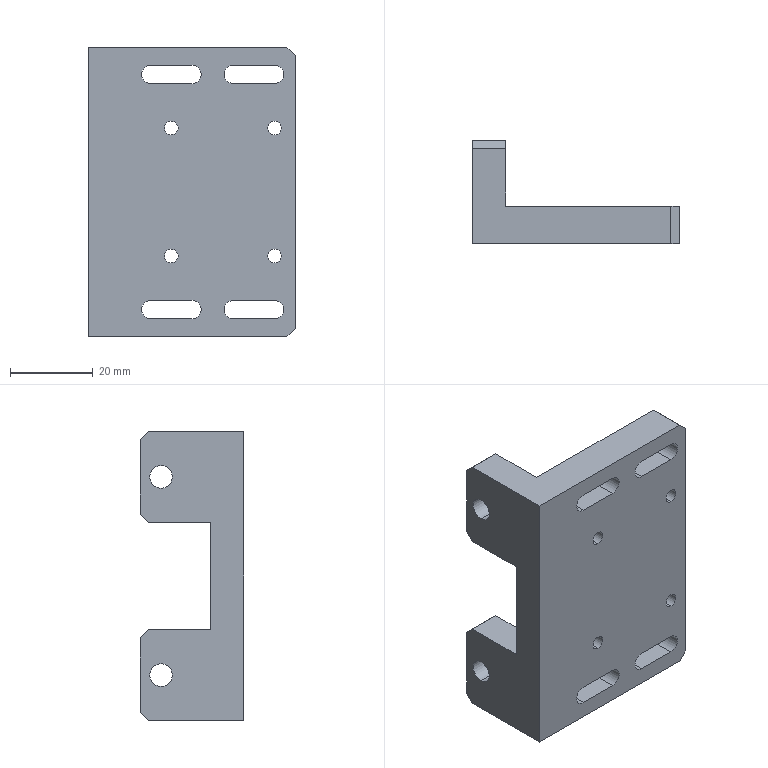Part | SolidWorks | features BaseBody 1 | 1 solid | 48 faces | box 50 x 25 x 70 mm | volume 32851 mm3 | plane 28 | cylinder 20 | commonest cylinder face diameters 3.3 x8 4.5 x8 5.5 x4
STEP:
#1=CARTESIAN_POINT('',(20.,0.,-21.15));
#2=VERTEX_POINT('',#1);
#3=CARTESIAN_POINT('',(20.,0.,-17.85));
#4=VERTEX_POINT('',#3);
#5=CARTESIAN_POINT('',(20.,0.,-19.5));
#6=DIRECTION('',(0.,1.,0.));
#7=DIRECTION('',(0.,0.,1.));
#8=AXIS2_PLACEMENT_3D('',#5,#6,#7);
#9=CIRCLE('',#8,1.65);
#10=EDGE_CURVE('',#2,#4,#9,.T.);
#11=ORIENTED_EDGE('',*,*,#10,.F.);
#12=CARTESIAN_POINT('',(20.,9.,-21.15));
#13=VERTEX_POINT('',#12);
#14=CARTESIAN_POINT('',(20.,9.,-21.15));
#15=DIRECTION('',(0.,1.,0.));
#16=VECTOR('',#15,1000.);
#17=LINE('',#14,#16);
#18=EDGE_CURVE('',#2,#13,#17,.T.);
#19=ORIENTED_EDGE('',*,*,#18,.T.);
#20=CARTESIAN_POINT('',(20.,9.,-17.85));
#21=VERTEX_POINT('',#20);
#22=CARTESIAN_POINT('',(20.,9.,-19.5));
#23=DIRECTION('',(0.,-1.,0.));
#24=DIRECTION('',(0.,0.,1.));
#25=AXIS2_PLACEMENT_3D('',#22,#23,#24);
#26=CIRCLE('',#25,1.65);
#27=EDGE_CURVE('',#21,#13,#26,.T.);
#28=ORIENTED_EDGE('',*,*,#27,.F.);
#29=CARTESIAN_POINT('',(20.,9.,-17.85));
#30=DIRECTION('',(0.,1.,0.));
#31=VECTOR('',#30,1000.);
#32=LINE('',#29,#31);
#33=EDGE_CURVE('',#4,#21,#32,.T.);
#34=ORIENTED_EDGE('',*,*,#33,.F.);
#35=EDGE_LOOP('',(#11,#19,#28,#34));
#36=FACE_OUTER_BOUND('',#35,.T.);
#37=CARTESIAN_POINT('',(20.,9.,-19.5));
#38=DIRECTION('',(0.,1.,0.));
#39=DIRECTION('',(0.,0.,1.));
#40=AXIS2_PLACEMENT_3D('',#37,#38,#39);
#41=CYLINDRICAL_SURFACE('',#40,1.65);
#42=ADVANCED_FACE('',(#36),#41,.F.);
#43=CARTESIAN_POINT('',(45.,0.,-21.15));
#44=VERTEX_POINT('',#43);
#45=CARTESIAN_POINT('',(45.,0.,-17.85));
#46=VERTEX_POINT('',#45);
#47=CARTESIAN_POINT('',(45.,0.,-19.5));
#48=DIRECTION('',(0.,1.,0.));
#49=DIRECTION('',(0.,0.,1.));
#50=AXIS2_PLACEMENT_3D('',#47,#48,#49);
#51=CIRCLE('',#50,1.65);
#52=EDGE_CURVE('',#44,#46,#51,.T.);
#53=ORIENTED_EDGE('',*,*,#52,.F.);
#54=CARTESIAN_POINT('',(45.,9.,-21.15));
#55=VERTEX_POINT('',#54);
#56=CARTESIAN_POINT('',(45.,9.,-21.15));
#57=DIRECTION('',(0.,1.,0.));
#58=VECTOR('',#57,1000.);
#59=LINE('',#56,#58);
#60=EDGE_CURVE('',#44,#55,#59,.T.);
#61=ORIENTED_EDGE('',*,*,#60,.T.);
#62=CARTESIAN_POINT('',(45.,9.,-17.85));
#63=VERTEX_POINT('',#62);
#64=CARTESIAN_POINT('',(45.,9.,-19.5));
#65=DIRECTION('',(0.,-1.,0.));
#66=DIRECTION('',(0.,0.,1.));
#67=AXIS2_PLACEMENT_3D('',#64,#65,#66);
#68=CIRCLE('',#67,1.65);
#69=EDGE_CURVE('',#63,#55,#68,.T.);
#70=ORIENTED_EDGE('',*,*,#69,.F.);
#71=CARTESIAN_POINT('',(45.,9.,-17.85));
#72=DIRECTION('',(0.,1.,0.));
#73=VECTOR('',#72,1000.);
#74=LINE('',#71,#73);
#75=EDGE_CURVE('',#46,#63,#74,.T.);
#76=ORIENTED_EDGE('',*,*,#75,.F.);
#77=EDGE_LOOP('',(#53,#61,#70,#76));
#78=FACE_OUTER_BOUND('',#77,.T.);
#79=CARTESIAN_POINT('',(45.,9.,-19.5));
#80=DIRECTION('',(0.,1.,0.));
#81=DIRECTION('',(0.,0.,1.));
#82=AXIS2_PLACEMENT_3D('',#79,#80,#81);
#83=CYLINDRICAL_SURFACE('',#82,1.65);
#84=ADVANCED_FACE('',(#78),#83,.F.);
#85=CARTESIAN_POINT('',(45.,0.,-52.15));
#86=VERTEX_POINT('',#85);
#87=CARTESIAN_POINT('',(45.,0.,-48.85));
#88=VERTEX_POINT('',#87);
#89=CARTESIAN_POINT('',(45.,0.,-50.5));
#90=DIRECTION('',(0.,1.,0.));
#91=DIRECTION('',(0.,0.,1.));
#92=AXIS2_PLACEMENT_3D('',#89,#90,#91);
#93=CIRCLE('',#92,1.65);
#94=EDGE_CURVE('',#86,#88,#93,.T.);
#95=ORIENTED_EDGE('',*,*,#94,.F.);
#96=CARTESIAN_POINT('',(45.,9.,-52.15));
#97=VERTEX_POINT('',#96);
#98=CARTESIAN_POINT('',(45.,9.,-52.15));
#99=DIRECTION('',(0.,1.,0.));
#100=VECTOR('',#99,1000.);
#101=LINE('',#98,#100);
#102=EDGE_CURVE('',#86,#97,#101,.T.);
#103=ORIENTED_EDGE('',*,*,#102,.T.);
#104=CARTESIAN_POINT('',(45.,9.,-48.85));
#105=VERTEX_POINT('',#104);
#106=CARTESIAN_POINT('',(45.,9.,-50.5));
#107=DIRECTION('',(0.,-1.,0.));
#108=DIRECTION('',(0.,0.,1.));
#109=AXIS2_PLACEMENT_3D('',#106,#107,#108);
#110=CIRCLE('',#109,1.65);
#111=EDGE_CURVE('',#105,#97,#110,.T.);
#112=ORIENTED_EDGE('',*,*,#111,.F.);
#113=CARTESIAN_POINT('',(45.,9.,-48.85));
#114=DIRECTION('',(0.,1.,0.));
#115=VECTOR('',#114,1000.);
#116=LINE('',#113,#115);
#117=EDGE_CURVE('',#88,#105,#116,.T.);
#118=ORIENTED_EDGE('',*,*,#117,.F.);
#119=EDGE_LOOP('',(#95,#103,#112,#118));
#120=FACE_OUTER_BOUND('',#119,.T.);
#121=CARTESIAN_POINT('',(45.,9.,-50.5));
#122=DIRECTION('',(0.,1.,0.));
#123=DIRECTION('',(0.,0.,1.));
#124=AXIS2_PLACEMENT_3D('',#121,#122,#123);
#125=CYLINDRICAL_SURFACE('',#124,1.65);
#126=ADVANCED_FACE('',(#120),#125,.F.);
#127=CARTESIAN_POINT('',(20.,0.,-52.15));
#128=VERTEX_POINT('',#127);
#129=CARTESIAN_POINT('',(20.,0.,-48.85));
#130=VERTEX_POINT('',#129);
#131=CARTESIAN_POINT('',(20.,0.,-50.5));
#132=DIRECTION('',(0.,1.,0.));
#133=DIRECTION('',(0.,0.,1.));
#134=AXIS2_PLACEMENT_3D('',#131,#132,#133);
#135=CIRCLE('',#134,1.65);
#136=EDGE_CURVE('',#128,#130,#135,.T.);
#137=ORIENTED_EDGE('',*,*,#136,.F.);
#138=CARTESIAN_POINT('',(20.,9.,-52.15));
#139=VERTEX_POINT('',#138);
#140=CARTESIAN_POINT('',(20.,9.,-52.15));
#141=DIRECTION('',(0.,1.,0.));
#142=VECTOR('',#141,1000.);
#143=LINE('',#140,#142);
#144=EDGE_CURVE('',#128,#139,#143,.T.);
#145=ORIENTED_EDGE('',*,*,#144,.T.);
#146=CARTESIAN_POINT('',(20.,9.,-48.85));
#147=VERTEX_POINT('',#146);
#148=CARTESIAN_POINT('',(20.,9.,-50.5));
#149=DIRECTION('',(0.,-1.,0.));
#150=DIRECTION('',(0.,0.,1.));
#151=AXIS2_PLACEMENT_3D('',#148,#149,#150);
#152=CIRCLE('',#151,1.65);
#153=EDGE_CURVE('',#147,#139,#152,.T.);
#154=ORIENTED_EDGE('',*,*,#153,.F.);
#155=CARTESIAN_POINT('',(20.,9.,-48.85));
#156=DIRECTION('',(0.,1.,0.));
#157=VECTOR('',#156,1000.);
#158=LINE('',#155,#157);
#159=EDGE_CURVE('',#130,#147,#158,.T.);
#160=ORIENTED_EDGE('',*,*,#159,.F.);
#161=EDGE_LOOP('',(#137,#145,#154,#160));
#162=FACE_OUTER_BOUND('',#161,.T.);
#163=CARTESIAN_POINT('',(20.,9.,-50.5));
#164=DIRECTION('',(0.,1.,0.));
#165=DIRECTION('',(0.,0.,1.));
#166=AXIS2_PLACEMENT_3D('',#163,#164,#165);
#167=CYLINDRICAL_SURFACE('',#166,1.65);
#168=ADVANCED_FACE('',(#162),#167,.F.);
#169=CARTESIAN_POINT('',(0.,20.,-61.75));
#170=VERTEX_POINT('',#169);
#171=CARTESIAN_POINT('',(0.,20.,-56.25));
#172=VERTEX_POINT('',#171);
#173=CARTESIAN_POINT('',(0.,20.,-59.));
#174=DIRECTION('',(-1.,0.,0.));
#175=DIRECTION('',(0.,0.,-1.));
#176=AXIS2_PLACEMENT_3D('',#173,#174,#175);
#177=CIRCLE('',#176,2.75);
#178=EDGE_CURVE('',#170,#172,#177,.T.);
#179=ORIENTED_EDGE('',*,*,#178,.T.);
#180=CARTESIAN_POINT('',(8.,20.,-56.25));
#181=VERTEX_POINT('',#180);
#182=CARTESIAN_POINT('',(8.,20.,-56.25));
#183=DIRECTION('',(1.,0.,0.));
#184=VECTOR('',#183,1000.);
#185=LINE('',#182,#184);
#186=EDGE_CURVE('',#172,#181,#185,.T.);
#187=ORIENTED_EDGE('',*,*,#186,.T.);
#188=CARTESIAN_POINT('',(8.,20.,-61.75));
#189=VERTEX_POINT('',#188);
#190=CARTESIAN_POINT('',(8.,20.,-59.));
#191=DIRECTION('',(-1.,0.,0.));
#192=DIRECTION('',(0.,0.,-1.));
#193=AXIS2_PLACEMENT_3D('',#190,#191,#192);
#194=CIRCLE('',#193,2.75);
#195=EDGE_CURVE('',#189,#181,#194,.T.);
#196=ORIENTED_EDGE('',*,*,#195,.F.);
#197=CARTESIAN_POINT('',(8.,20.,-61.75));
#198=DIRECTION('',(1.,0.,0.));
#199=VECTOR('',#198,1000.);
#200=LINE('',#197,#199);
#201=EDGE_CURVE('',#170,#189,#200,.T.);
#202=ORIENTED_EDGE('',*,*,#201,.F.);
#203=EDGE_LOOP('',(#179,#187,#196,#202));
#204=FACE_OUTER_BOUND('',#203,.T.);
#205=CARTESIAN_POINT('',(8.,20.,-59.));
#206=DIRECTION('',(1.,0.,0.));
#207=DIRECTION('',(0.,0.,-1.));
#208=AXIS2_PLACEMENT_3D('',#205,#206,#207);
#209=CYLINDRICAL_SURFACE('',#208,2.75);
#210=ADVANCED_FACE('',(#204),#209,.F.);
#211=CARTESIAN_POINT('',(0.,20.,-13.75));
#212=VERTEX_POINT('',#211);
#213=CARTESIAN_POINT('',(0.,20.,-8.25));
#214=VERTEX_POINT('',#213);
#215=CARTESIAN_POINT('',(0.,20.,-11.));
#216=DIRECTION('',(-1.,0.,0.));
#217=DIRECTION('',(0.,0.,-1.));
#218=AXIS2_PLACEMENT_3D('',#215,#216,#217);
#219=CIRCLE('',#218,2.75);
#220=EDGE_CURVE('',#212,#214,#219,.T.);
#221=ORIENTED_EDGE('',*,*,#220,.T.);
#222=CARTESIAN_POINT('',(8.,20.,-8.25));
#223=VERTEX_POINT('',#222);
#224=CARTESIAN_POINT('',(8.,20.,-8.25));
#225=DIRECTION('',(1.,0.,0.));
#226=VECTOR('',#225,1000.);
#227=LINE('',#224,#226);
#228=EDGE_CURVE('',#214,#223,#227,.T.);
#229=ORIENTED_EDGE('',*,*,#228,.T.);
#230=CARTESIAN_POINT('',(8.,20.,-13.75));
#231=VERTEX_POINT('',#230);
#232=CARTESIAN_POINT('',(8.,20.,-11.));
#233=DIRECTION('',(-1.,0.,0.));
#234=DIRECTION('',(0.,0.,-1.));
#235=AXIS2_PLACEMENT_3D('',#232,#233,#234);
#236=CIRCLE('',#235,2.75);
#237=EDGE_CURVE('',#231,#223,#236,.T.);
#238=ORIENTED_EDGE('',*,*,#237,.F.);
#239=CARTESIAN_POINT('',(8.,20.,-13.75));
#240=DIRECTION('',(1.,0.,0.));
#241=VECTOR('',#240,1000.);
#242=LINE('',#239,#241);
#243=EDGE_CURVE('',#212,#231,#242,.T.);
#244=ORIENTED_EDGE('',*,*,#243,.F.);
#245=EDGE_LOOP('',(#221,#229,#238,#244));
#246=FACE_OUTER_BOUND('',#245,.T.);
#247=CARTESIAN_POINT('',(8.,20.,-11.));
#248=DIRECTION('',(1.,0.,0.));
#249=DIRECTION('',(0.,0.,-1.));
#250=AXIS2_PLACEMENT_3D('',#247,#248,#249);
#251=CYLINDRICAL_SURFACE('',#250,2.75);
#252=ADVANCED_FACE('',(#246),#251,.F.);
#253=CARTESIAN_POINT('',(20.,0.,-19.5));
#254=DIRECTION('',(0.,1.,0.));
#255=DIRECTION('',(0.,0.,1.));
#256=AXIS2_PLACEMENT_3D('',#253,#254,#255);
#257=CIRCLE('',#256,1.65);
#258=EDGE_CURVE('',#4,#2,#257,.T.);
#259=ORIENTED_EDGE('',*,*,#258,.T.);
#260=ORIENTED_EDGE('',*,*,#10,.T.);
#261=EDGE_LOOP('',(#259,#260));
#262=FACE_BOUND('',#261,.T.);
#263=CARTESIAN_POINT('',(45.,0.,-19.5));
#264=DIRECTION('',(0.,1.,0.));
#265=DIRECTION('',(0.,0.,1.));
#266=AXIS2_PLACEMENT_3D('',#263,#264,#265);
#267=CIRCLE('',#266,1.65);
#268=EDGE_CURVE('',#46,#44,#267,.T.);
#269=ORIENTED_EDGE('',*,*,#268,.T.);
#270=ORIENTED_EDGE('',*,*,#52,.T.);
#271=EDGE_LOOP('',(#269,#270));
#272=FACE_BOUND('',#271,.T.);
#273=CARTESIAN_POINT('',(45.,0.,-50.5));
#274=DIRECTION('',(0.,1.,0.));
#275=DIRECTION('',(0.,0.,1.));
#276=AXIS2_PLACEMENT_3D('',#273,#274,#275);
#277=CIRCLE('',#276,1.65);
#278=EDGE_CURVE('',#88,#86,#277,.T.);
#279=ORIENTED_EDGE('',*,*,#278,.T.);
#280=ORIENTED_EDGE('',*,*,#94,.T.);
#281=EDGE_LOOP('',(#279,#280));
#282=FACE_BOUND('',#281,.T.);
#283=CARTESIAN_POINT('',(20.,0.,-50.5));
#284=DIRECTION('',(0.,1.,0.));
#285=DIRECTION('',(0.,0.,1.));
#286=AXIS2_PLACEMENT_3D('',#283,#284,#285);
#287=CIRCLE('',#286,1.65);
#288=EDGE_CURVE('',#130,#128,#287,.T.);
#289=ORIENTED_EDGE('',*,*,#288,.T.);
#290=ORIENTED_EDGE('',*,*,#136,.T.);
#291=EDGE_LOOP('',(#289,#290));
#292=FACE_BOUND('',#291,.T.);
#293=CARTESIAN_POINT('',(25.,0.,-61.25));
#294=VERTEX_POINT('',#293);
#295=CARTESIAN_POINT('',(25.,0.,-65.75));
#296=VERTEX_POINT('',#295);
#297=CARTESIAN_POINT('',(25.,0.,-63.5));
#298=DIRECTION('',(0.,1.,0.));
#299=DIRECTION('',(0.,0.,1.));
#300=AXIS2_PLACEMENT_3D('',#297,#298,#299);
#301=CIRCLE('',#300,2.25);
#302=EDGE_CURVE('',#294,#296,#301,.T.);
#303=ORIENTED_EDGE('',*,*,#302,.T.);
#304=CARTESIAN_POINT('',(15.,0.,-65.75));
#305=VERTEX_POINT('',#304);
#306=CARTESIAN_POINT('',(0.,0.,-65.75));
#307=DIRECTION('',(-1.,0.,0.));
#308=VECTOR('',#307,1000.);
#309=LINE('',#306,#308);
#310=EDGE_CURVE('',#296,#305,#309,.T.);
#311=ORIENTED_EDGE('',*,*,#310,.T.);
#312=CARTESIAN_POINT('',(15.,0.,-61.25));
#313=VERTEX_POINT('',#312);
#314=CARTESIAN_POINT('',(15.,0.,-63.5));
#315=DIRECTION('',(0.,1.,0.));
#316=DIRECTION('',(0.,0.,1.));
#317=AXIS2_PLACEMENT_3D('',#314,#315,#316);
#318=CIRCLE('',#317,2.25);
#319=EDGE_CURVE('',#305,#313,#318,.T.);
#320=ORIENTED_EDGE('',*,*,#319,.T.);
#321=CARTESIAN_POINT('',(0.,0.,-61.25));
#322=DIRECTION('',(1.,0.,0.));
#323=VECTOR('',#322,1000.);
#324=LINE('',#321,#323);
#325=EDGE_CURVE('',#313,#294,#324,.T.);
#326=ORIENTED_EDGE('',*,*,#325,.T.);
#327=EDGE_LOOP('',(#303,#311,#320,#326));
#328=FACE_BOUND('',#327,.T.);
#329=CARTESIAN_POINT('',(45.,0.,-61.25));
#330=VERTEX_POINT('',#329);
#331=CARTESIAN_POINT('',(45.,0.,-65.75));
#332=VERTEX_POINT('',#331);
#333=CARTESIAN_POINT('',(45.,0.,-63.5));
#334=DIRECTION('',(0.,1.,0.));
#335=DIRECTION('',(0.,0.,1.));
#336=AXIS2_PLACEMENT_3D('',#333,#334,#335);
#337=CIRCLE('',#336,2.25);
#338=EDGE_CURVE('',#330,#332,#337,.T.);
#339=ORIENTED_EDGE('',*,*,#338,.T.);
#340=CARTESIAN_POINT('',(35.,0.,-65.75));
#341=VERTEX_POINT('',#340);
#342=CARTESIAN_POINT('',(0.,0.,-65.75));
#343=DIRECTION('',(-1.,0.,0.));
#344=VECTOR('',#343,1000.);
#345=LINE('',#342,#344);
#346=EDGE_CURVE('',#332,#341,#345,.T.);
#347=ORIENTED_EDGE('',*,*,#346,.T.);
#348=CARTESIAN_POINT('',(35.,0.,-61.25));
#349=VERTEX_POINT('',#348);
#350=CARTESIAN_POINT('',(35.,0.,-63.5));
#351=DIRECTION('',(0.,1.,0.));
#352=DIRECTION('',(0.,0.,1.));
#353=AXIS2_PLACEMENT_3D('',#350,#351,#352);
#354=CIRCLE('',#353,2.25);
#355=EDGE_CURVE('',#341,#349,#354,.T.);
#356=ORIENTED_EDGE('',*,*,#355,.T.);
#357=CARTESIAN_POINT('',(0.,0.,-61.25));
#358=DIRECTION('',(1.,0.,0.));
#359=VECTOR('',#358,1000.);
#360=LINE('',#357,#359);
#361=EDGE_CURVE('',#349,#330,#360,.T.);
#362=ORIENTED_EDGE('',*,*,#361,.T.);
#363=EDGE_LOOP('',(#339,#347,#356,#362));
#364=FACE_BOUND('',#363,.T.);
#365=CARTESIAN_POINT('',(45.,0.,-4.25));
#366=VERTEX_POINT('',#365);
#367=CARTESIAN_POINT('',(45.,0.,-8.75));
#368=VERTEX_POINT('',#367);
#369=CARTESIAN_POINT('',(45.,0.,-6.5));
#370=DIRECTION('',(0.,1.,0.));
#371=DIRECTION('',(0.,0.,1.));
#372=AXIS2_PLACEMENT_3D('',#369,#370,#371);
#373=CIRCLE('',#372,2.25);
#374=EDGE_CURVE('',#366,#368,#373,.T.);
#375=ORIENTED_EDGE('',*,*,#374,.T.);
#376=CARTESIAN_POINT('',(35.,0.,-8.75));
#377=VERTEX_POINT('',#376);
#378=CARTESIAN_POINT('',(0.,0.,-8.75));
#379=DIRECTION('',(-1.,0.,0.));
#380=VECTOR('',#379,1000.);
#381=LINE('',#378,#380);
#382=EDGE_CURVE('',#368,#377,#381,.T.);
#383=ORIENTED_EDGE('',*,*,#382,.T.);
#384=CARTESIAN_POINT('',(35.,0.,-4.25));
#385=VERTEX_POINT('',#384);
#386=CARTESIAN_POINT('',(35.,0.,-6.5));
#387=DIRECTION('',(0.,1.,0.));
#388=DIRECTION('',(0.,0.,1.));
#389=AXIS2_PLACEMENT_3D('',#386,#387,#388);
#390=CIRCLE('',#389,2.25);
#391=EDGE_CURVE('',#377,#385,#390,.T.);
#392=ORIENTED_EDGE('',*,*,#391,.T.);
#393=CARTESIAN_POINT('',(0.,0.,-4.25));
#394=DIRECTION('',(1.,0.,0.));
#395=VECTOR('',#394,1000.);
#396=LINE('',#393,#395);
#397=EDGE_CURVE('',#385,#366,#396,.T.);
#398=ORIENTED_EDGE('',*,*,#397,.T.);
#399=EDGE_LOOP('',(#375,#383,#392,#398));
#400=FACE_BOUND('',#399,.T.);
#401=CARTESIAN_POINT('',(25.,0.,-4.25));
#402=VERTEX_POINT('',#401);
#403=CARTESIAN_POINT('',(25.,0.,-8.75));
#404=VERTEX_POINT('',#403);
#405=CARTESIAN_POINT('',(25.,0.,-6.5));
#406=DIRECTION('',(0.,1.,0.));
#407=DIRECTION('',(0.,0.,1.));
#408=AXIS2_PLACEMENT_3D('',#405,#406,#407);
#409=CIRCLE('',#408,2.25);
#410=EDGE_CURVE('',#402,#404,#409,.T.);
#411=ORIENTED_EDGE('',*,*,#410,.T.);
#412=CARTESIAN_POINT('',(15.,0.,-8.75));
#413=VERTEX_POINT('',#412);
#414=CARTESIAN_POINT('',(0.,0.,-8.75));
#415=DIRECTION('',(-1.,0.,0.));
#416=VECTOR('',#415,1000.);
#417=LINE('',#414,#416);
#418=EDGE_CURVE('',#404,#413,#417,.T.);
#419=ORIENTED_EDGE('',*,*,#418,.T.);
#420=CARTESIAN_POINT('',(15.,0.,-4.25));
#421=VERTEX_POINT('',#420);
#422=CARTESIAN_POINT('',(15.,0.,-6.5));
#423=DIRECTION('',(0.,1.,0.));
#424=DIRECTION('',(0.,0.,1.));
#425=AXIS2_PLACEMENT_3D('',#422,#423,#424);
#426=CIRCLE('',#425,2.25);
#427=EDGE_CURVE('',#413,#421,#426,.T.);
#428=ORIENTED_EDGE('',*,*,#427,.T.);
#429=CARTESIAN_POINT('',(0.,0.,-4.25));
#430=DIRECTION('',(1.,0.,0.));
#431=VECTOR('',#430,1000.);
#432=LINE('',#429,#431);
#433=EDGE_CURVE('',#421,#402,#432,.T.);
#434=ORIENTED_EDGE('',*,*,#433,.T.);
#435=EDGE_LOOP('',(#411,#419,#428,#434));
#436=FACE_BOUND('',#435,.T.);
#437=CARTESIAN_POINT('',(0.,0.,-70.));
#438=VERTEX_POINT('',#437);
#439=CARTESIAN_POINT('',(48.,0.,-70.));
#440=VERTEX_POINT('',#439);
#441=CARTESIAN_POINT('',(0.,0.,-70.));
#442=DIRECTION('',(1.,0.,0.));
#443=VECTOR('',#442,1000.);
#444=LINE('',#441,#443);
#445=EDGE_CURVE('',#438,#440,#444,.T.);
#446=ORIENTED_EDGE('',*,*,#445,.T.);
#447=CARTESIAN_POINT('',(50.,0.,-68.));
#448=VERTEX_POINT('',#447);
#449=CARTESIAN_POINT('',(48.,0.,-70.));
#450=DIRECTION('',(0.7071,0.,0.7071));
#451=VECTOR('',#450,1000.);
#452=LINE('',#449,#451);
#453=EDGE_CURVE('',#440,#448,#452,.T.);
#454=ORIENTED_EDGE('',*,*,#453,.T.);
#455=CARTESIAN_POINT('',(50.,0.,-2.));
#456=VERTEX_POINT('',#455);
#457=CARTESIAN_POINT('',(50.,0.,0.));
#458=DIRECTION('',(0.,0.,1.));
#459=VECTOR('',#458,1000.);
#460=LINE('',#457,#459);
#461=EDGE_CURVE('',#448,#456,#460,.T.);
#462=ORIENTED_EDGE('',*,*,#461,.T.);
#463=CARTESIAN_POINT('',(48.,0.,0.));
#464=VERTEX_POINT('',#463);
#465=CARTESIAN_POINT('',(50.,0.,-2.));
#466=DIRECTION('',(-0.7071,0.,0.7071));
#467=VECTOR('',#466,1000.);
#468=LINE('',#465,#467);
#469=EDGE_CURVE('',#456,#464,#468,.T.);
#470=ORIENTED_EDGE('',*,*,#469,.T.);
#471=CARTESIAN_POINT('',(0.,0.,0.));
#472=VERTEX_POINT('',#471);
#473=CARTESIAN_POINT('',(0.,0.,0.));
#474=DIRECTION('',(-1.,0.,0.));
#475=VECTOR('',#474,1000.);
#476=LINE('',#473,#475);
#477=EDGE_CURVE('',#464,#472,#476,.T.);
#478=ORIENTED_EDGE('',*,*,#477,.T.);
#479=CARTESIAN_POINT('',(0.,0.,0.));
#480=DIRECTION('',(0.,0.,-1.));
#481=VECTOR('',#480,1000.);
#482=LINE('',#479,#481);
#483=EDGE_CURVE('',#472,#438,#482,.T.);
#484=ORIENTED_EDGE('',*,*,#483,.T.);
#485=EDGE_LOOP('',(#446,#454,#462,#470,#478,#484));
#486=FACE_OUTER_BOUND('',#485,.T.);
#487=CARTESIAN_POINT('',(0.,0.,0.));
#488=DIRECTION('',(0.,-1.,0.));
#489=DIRECTION('',(0.,0.,-1.));
#490=AXIS2_PLACEMENT_3D('',#487,#488,#489);
#491=PLANE('',#490);
#492=ADVANCED_FACE('',(#262,#272,#282,#292,#328,#364,#400,#436,#486),#491,.T.);
#493=ORIENTED_EDGE('',*,*,#18,.F.);
#494=ORIENTED_EDGE('',*,*,#258,.F.);
#495=ORIENTED_EDGE('',*,*,#33,.T.);
#496=CARTESIAN_POINT('',(20.,9.,-19.5));
#497=DIRECTION('',(0.,-1.,0.));
#498=DIRECTION('',(0.,0.,1.));
#499=AXIS2_PLACEMENT_3D('',#496,#497,#498);
#500=CIRCLE('',#499,1.65);
#501=EDGE_CURVE('',#13,#21,#500,.T.);
#502=ORIENTED_EDGE('',*,*,#501,.F.);
#503=EDGE_LOOP('',(#493,#494,#495,#502));
#504=FACE_OUTER_BOUND('',#503,.T.);
#505=CARTESIAN_POINT('',(20.,9.,-19.5));
#506=DIRECTION('',(0.,1.,0.));
#507=DIRECTION('',(0.,0.,1.));
#508=AXIS2_PLACEMENT_3D('',#505,#506,#507);
#509=CYLINDRICAL_SURFACE('',#508,1.65);
#510=ADVANCED_FACE('',(#504),#509,.F.);
#511=ORIENTED_EDGE('',*,*,#60,.F.);
#512=ORIENTED_EDGE('',*,*,#268,.F.);
#513=ORIENTED_EDGE('',*,*,#75,.T.);
#514=CARTESIAN_POINT('',(45.,9.,-19.5));
#515=DIRECTION('',(0.,-1.,0.));
#516=DIRECTION('',(0.,0.,1.));
#517=AXIS2_PLACEMENT_3D('',#514,#515,#516);
#518=CIRCLE('',#517,1.65);
#519=EDGE_CURVE('',#55,#63,#518,.T.);
#520=ORIENTED_EDGE('',*,*,#519,.F.);
#521=EDGE_LOOP('',(#511,#512,#513,#520));
#522=FACE_OUTER_BOUND('',#521,.T.);
#523=CARTESIAN_POINT('',(45.,9.,-19.5));
#524=DIRECTION('',(0.,1.,0.));
#525=DIRECTION('',(0.,0.,1.));
#526=AXIS2_PLACEMENT_3D('',#523,#524,#525);
#527=CYLINDRICAL_SURFACE('',#526,1.65);
#528=ADVANCED_FACE('',(#522),#527,.F.);
#529=ORIENTED_EDGE('',*,*,#102,.F.);
#530=ORIENTED_EDGE('',*,*,#278,.F.);
#531=ORIENTED_EDGE('',*,*,#117,.T.);
#532=CARTESIAN_POINT('',(45.,9.,-50.5));
#533=DIRECTION('',(0.,-1.,0.));
#534=DIRECTION('',(0.,0.,1.));
#535=AXIS2_PLACEMENT_3D('',#532,#533,#534);
#536=CIRCLE('',#535,1.65);
#537=EDGE_CURVE('',#97,#105,#536,.T.);
#538=ORIENTED_EDGE('',*,*,#537,.F.);
#539=EDGE_LOOP('',(#529,#530,#531,#538));
#540=FACE_OUTER_BOUND('',#539,.T.);
#541=CARTESIAN_POINT('',(45.,9.,-50.5));
#542=DIRECTION('',(0.,1.,0.));
#543=DIRECTION('',(0.,0.,1.));
#544=AXIS2_PLACEMENT_3D('',#541,#542,#543);
#545=CYLINDRICAL_SURFACE('',#544,1.65);
#546=ADVANCED_FACE('',(#540),#545,.F.);
#547=ORIENTED_EDGE('',*,*,#144,.F.);
#548=ORIENTED_EDGE('',*,*,#288,.F.);
#549=ORIENTED_EDGE('',*,*,#159,.T.);
#550=CARTESIAN_POINT('',(20.,9.,-50.5));
#551=DIRECTION('',(0.,-1.,0.));
#552=DIRECTION('',(0.,0.,1.));
#553=AXIS2_PLACEMENT_3D('',#550,#551,#552);
#554=CIRCLE('',#553,1.65);
#555=EDGE_CURVE('',#139,#147,#554,.T.);
#556=ORIENTED_EDGE('',*,*,#555,.F.);
#557=EDGE_LOOP('',(#547,#548,#549,#556));
#558=FACE_OUTER_BOUND('',#557,.T.);
#559=CARTESIAN_POINT('',(20.,9.,-50.5));
#560=DIRECTION('',(0.,1.,0.));
#561=DIRECTION('',(0.,0.,1.));
#562=AXIS2_PLACEMENT_3D('',#559,#560,#561);
#563=CYLINDRICAL_SURFACE('',#562,1.65);
#564=ADVANCED_FACE('',(#558),#563,.F.);
#565=CARTESIAN_POINT('',(15.,9.,-65.75));
#566=VERTEX_POINT('',#565);
#567=CARTESIAN_POINT('',(15.,0.,-65.75));
#568=DIRECTION('',(0.,1.,0.));
#569=VECTOR('',#568,1000.);
#570=LINE('',#567,#569);
#571=EDGE_CURVE('',#305,#566,#570,.T.);
#572=ORIENTED_EDGE('',*,*,#571,.F.);
#573=ORIENTED_EDGE('',*,*,#310,.F.);
#574=CARTESIAN_POINT('',(25.,9.,-65.75));
#575=VERTEX_POINT('',#574);
#576=CARTESIAN_POINT('',(25.,0.,-65.75));
#577=DIRECTION('',(0.,-1.,0.));
#578=VECTOR('',#577,1000.);
#579=LINE('',#576,#578);
#580=EDGE_CURVE('',#575,#296,#579,.T.);
#581=ORIENTED_EDGE('',*,*,#580,.F.);
#582=CARTESIAN_POINT('',(15.,9.,-65.75));
#583=DIRECTION('',(1.,0.,0.));
#584=VECTOR('',#583,1000.);
#585=LINE('',#582,#584);
#586=EDGE_CURVE('',#566,#575,#585,.T.);
#587=ORIENTED_EDGE('',*,*,#586,.F.);
#588=EDGE_LOOP('',(#572,#573,#581,#587));
#589=FACE_OUTER_BOUND('',#588,.T.);
#590=CARTESIAN_POINT('',(15.,0.,-65.75));
#591=DIRECTION('',(0.,0.,-1.));
#592=DIRECTION('',(-1.,0.,0.));
#593=AXIS2_PLACEMENT_3D('',#590,#591,#592);
#594=PLANE('',#593);
#595=ADVANCED_FACE('',(#589),#594,.F.);
#596=ORIENTED_EDGE('',*,*,#580,.T.);
#597=ORIENTED_EDGE('',*,*,#302,.F.);
#598=CARTESIAN_POINT('',(25.,9.,-61.25));
#599=VERTEX_POINT('',#598);
#600=CARTESIAN_POINT('',(25.,0.,-61.25));
#601=DIRECTION('',(0.,-1.,0.));
#602=VECTOR('',#601,1000.);
#603=LINE('',#600,#602);
#604=EDGE_CURVE('',#599,#294,#603,.T.);
#605=ORIENTED_EDGE('',*,*,#604,.F.);
#606=CARTESIAN_POINT('',(25.,9.,-63.5));
#607=DIRECTION('',(0.,-1.,0.));
#608=DIRECTION('',(0.,0.,1.));
#609=AXIS2_PLACEMENT_3D('',#606,#607,#608);
#610=CIRCLE('',#609,2.25);
#611=EDGE_CURVE('',#575,#599,#610,.T.);
#612=ORIENTED_EDGE('',*,*,#611,.F.);
#613=EDGE_LOOP('',(#596,#597,#605,#612));
#614=FACE_OUTER_BOUND('',#613,.T.);
#615=CARTESIAN_POINT('',(25.,0.,-63.5));
#616=DIRECTION('',(0.,1.,0.));
#617=DIRECTION('',(0.,0.,1.));
#618=AXIS2_PLACEMENT_3D('',#615,#616,#617);
#619=CYLINDRICAL_SURFACE('',#618,2.25);
#620=ADVANCED_FACE('',(#614),#619,.F.);
#621=ORIENTED_EDGE('',*,*,#604,.T.);
#622=ORIENTED_EDGE('',*,*,#325,.F.);
#623=CARTESIAN_POINT('',(15.,9.,-61.25));
#624=VERTEX_POINT('',#623);
#625=CARTESIAN_POINT('',(15.,0.,-61.25));
#626=DIRECTION('',(0.,-1.,0.));
#627=VECTOR('',#626,1000.);
#628=LINE('',#625,#627);
#629=EDGE_CURVE('',#624,#313,#628,.T.);
#630=ORIENTED_EDGE('',*,*,#629,.F.);
#631=CARTESIAN_POINT('',(15.,9.,-61.25));
#632=DIRECTION('',(-1.,0.,0.));
#633=VECTOR('',#632,1000.);
#634=LINE('',#631,#633);
#635=EDGE_CURVE('',#599,#624,#634,.T.);
#636=ORIENTED_EDGE('',*,*,#635,.F.);
#637=EDGE_LOOP('',(#621,#622,#630,#636));
#638=FACE_OUTER_BOUND('',#637,.T.);
#639=CARTESIAN_POINT('',(15.,0.,-61.25));
#640=DIRECTION('',(0.,0.,1.));
#641=DIRECTION('',(1.,0.,0.));
#642=AXIS2_PLACEMENT_3D('',#639,#640,#641);
#643=PLANE('',#642);
#644=ADVANCED_FACE('',(#638),#643,.F.);
#645=ORIENTED_EDGE('',*,*,#629,.T.);
#646=ORIENTED_EDGE('',*,*,#319,.F.);
#647=ORIENTED_EDGE('',*,*,#571,.T.);
#648=CARTESIAN_POINT('',(15.,9.,-63.5));
#649=DIRECTION('',(0.,-1.,0.));
#650=DIRECTION('',(0.,0.,1.));
#651=AXIS2_PLACEMENT_3D('',#648,#649,#650);
#652=CIRCLE('',#651,2.25);
#653=EDGE_CURVE('',#624,#566,#652,.T.);
#654=ORIENTED_EDGE('',*,*,#653,.F.);
#655=EDGE_LOOP('',(#645,#646,#647,#654));
#656=FACE_OUTER_BOUND('',#655,.T.);
#657=CARTESIAN_POINT('',(15.,0.,-63.5));
#658=DIRECTION('',(0.,1.,0.));
#659=DIRECTION('',(0.,0.,1.));
#660=AXIS2_PLACEMENT_3D('',#657,#658,#659);
#661=CYLINDRICAL_SURFACE('',#660,2.25);
#662=ADVANCED_FACE('',(#656),#661,.F.);
#663=CARTESIAN_POINT('',(35.,9.,-65.75));
#664=VERTEX_POINT('',#663);
#665=CARTESIAN_POINT('',(35.,0.,-65.75));
#666=DIRECTION('',(0.,1.,0.));
#667=VECTOR('',#666,1000.);
#668=LINE('',#665,#667);
#669=EDGE_CURVE('',#341,#664,#668,.T.);
#670=ORIENTED_EDGE('',*,*,#669,.F.);
#671=ORIENTED_EDGE('',*,*,#346,.F.);
#672=CARTESIAN_POINT('',(45.,9.,-65.75));
#673=VERTEX_POINT('',#672);
#674=CARTESIAN_POINT('',(45.,0.,-65.75));
#675=DIRECTION('',(0.,-1.,0.));
#676=VECTOR('',#675,1000.);
#677=LINE('',#674,#676);
#678=EDGE_CURVE('',#673,#332,#677,.T.);
#679=ORIENTED_EDGE('',*,*,#678,.F.);
#680=CARTESIAN_POINT('',(35.,9.,-65.75));
#681=DIRECTION('',(1.,0.,0.));
#682=VECTOR('',#681,1000.);
#683=LINE('',#680,#682);
#684=EDGE_CURVE('',#664,#673,#683,.T.);
#685=ORIENTED_EDGE('',*,*,#684,.F.);
#686=EDGE_LOOP('',(#670,#671,#679,#685));
#687=FACE_OUTER_BOUND('',#686,.T.);
#688=CARTESIAN_POINT('',(35.,0.,-65.75));
#689=DIRECTION('',(0.,0.,-1.));
#690=DIRECTION('',(-1.,0.,0.));
#691=AXIS2_PLACEMENT_3D('',#688,#689,#690);
#692=PLANE('',#691);
#693=ADVANCED_FACE('',(#687),#692,.F.);
#694=ORIENTED_EDGE('',*,*,#678,.T.);
#695=ORIENTED_EDGE('',*,*,#338,.F.);
#696=CARTESIAN_POINT('',(45.,9.,-61.25));
#697=VERTEX_POINT('',#696);
#698=CARTESIAN_POINT('',(45.,0.,-61.25));
#699=DIRECTION('',(0.,-1.,0.));
#700=VECTOR('',#699,1000.);
#701=LINE('',#698,#700);
#702=EDGE_CURVE('',#697,#330,#701,.T.);
#703=ORIENTED_EDGE('',*,*,#702,.F.);
#704=CARTESIAN_POINT('',(45.,9.,-63.5));
#705=DIRECTION('',(0.,-1.,0.));
#706=DIRECTION('',(0.,0.,1.));
#707=AXIS2_PLACEMENT_3D('',#704,#705,#706);
#708=CIRCLE('',#707,2.25);
#709=EDGE_CURVE('',#673,#697,#708,.T.);
#710=ORIENTED_EDGE('',*,*,#709,.F.);
#711=EDGE_LOOP('',(#694,#695,#703,#710));
#712=FACE_OUTER_BOUND('',#711,.T.);
#713=CARTESIAN_POINT('',(45.,0.,-63.5));
#714=DIRECTION('',(0.,1.,0.));
#715=DIRECTION('',(0.,0.,1.));
#716=AXIS2_PLACEMENT_3D('',#713,#714,#715);
#717=CYLINDRICAL_SURFACE('',#716,2.25);
#718=ADVANCED_FACE('',(#712),#717,.F.);
#719=ORIENTED_EDGE('',*,*,#702,.T.);
#720=ORIENTED_EDGE('',*,*,#361,.F.);
#721=CARTESIAN_POINT('',(35.,9.,-61.25));
#722=VERTEX_POINT('',#721);
#723=CARTESIAN_POINT('',(35.,0.,-61.25));
#724=DIRECTION('',(0.,-1.,0.));
#725=VECTOR('',#724,1000.);
#726=LINE('',#723,#725);
#727=EDGE_CURVE('',#722,#349,#726,.T.);
#728=ORIENTED_EDGE('',*,*,#727,.F.);
#729=CARTESIAN_POINT('',(35.,9.,-61.25));
#730=DIRECTION('',(-1.,0.,0.));
#731=VECTOR('',#730,1000.);
#732=LINE('',#729,#731);
#733=EDGE_CURVE('',#697,#722,#732,.T.);
#734=ORIENTED_EDGE('',*,*,#733,.F.);
#735=EDGE_LOOP('',(#719,#720,#728,#734));
#736=FACE_OUTER_BOUND('',#735,.T.);
#737=CARTESIAN_POINT('',(35.,0.,-61.25));
#738=DIRECTION('',(0.,0.,1.));
#739=DIRECTION('',(1.,0.,0.));
#740=AXIS2_PLACEMENT_3D('',#737,#738,#739);
#741=PLANE('',#740);
#742=ADVANCED_FACE('',(#736),#741,.F.);
#743=ORIENTED_EDGE('',*,*,#727,.T.);
#744=ORIENTED_EDGE('',*,*,#355,.F.);
#745=ORIENTED_EDGE('',*,*,#669,.T.);
#746=CARTESIAN_POINT('',(35.,9.,-63.5));
#747=DIRECTION('',(0.,-1.,0.));
#748=DIRECTION('',(0.,0.,1.));
#749=AXIS2_PLACEMENT_3D('',#746,#747,#748);
#750=CIRCLE('',#749,2.25);
#751=EDGE_CURVE('',#722,#664,#750,.T.);
#752=ORIENTED_EDGE('',*,*,#751,.F.);
#753=EDGE_LOOP('',(#743,#744,#745,#752));
#754=FACE_OUTER_BOUND('',#753,.T.);
#755=CARTESIAN_POINT('',(35.,0.,-63.5));
#756=DIRECTION('',(0.,1.,0.));
#757=DIRECTION('',(0.,0.,1.));
#758=AXIS2_PLACEMENT_3D('',#755,#756,#757);
#759=CYLINDRICAL_SURFACE('',#758,2.25);
#760=ADVANCED_FACE('',(#754),#759,.F.);
#761=CARTESIAN_POINT('',(35.,9.,-8.75));
#762=VERTEX_POINT('',#761);
#763=CARTESIAN_POINT('',(35.,0.,-8.75));
#764=DIRECTION('',(0.,1.,0.));
#765=VECTOR('',#764,1000.);
#766=LINE('',#763,#765);
#767=EDGE_CURVE('',#377,#762,#766,.T.);
#768=ORIENTED_EDGE('',*,*,#767,.F.);
#769=ORIENTED_EDGE('',*,*,#382,.F.);
#770=CARTESIAN_POINT('',(45.,9.,-8.75));
#771=VERTEX_POINT('',#770);
#772=CARTESIAN_POINT('',(45.,0.,-8.75));
#773=DIRECTION('',(0.,-1.,0.));
#774=VECTOR('',#773,1000.);
#775=LINE('',#772,#774);
#776=EDGE_CURVE('',#771,#368,#775,.T.);
#777=ORIENTED_EDGE('',*,*,#776,.F.);
#778=CARTESIAN_POINT('',(35.,9.,-8.75));
#779=DIRECTION('',(1.,0.,0.));
#780=VECTOR('',#779,1000.);
#781=LINE('',#778,#780);
#782=EDGE_CURVE('',#762,#771,#781,.T.);
#783=ORIENTED_EDGE('',*,*,#782,.F.);
#784=EDGE_LOOP('',(#768,#769,#777,#783));
#785=FACE_OUTER_BOUND('',#784,.T.);
#786=CARTESIAN_POINT('',(35.,0.,-8.75));
#787=DIRECTION('',(0.,0.,-1.));
#788=DIRECTION('',(-1.,0.,0.));
#789=AXIS2_PLACEMENT_3D('',#786,#787,#788);
#790=PLANE('',#789);
#791=ADVANCED_FACE('',(#785),#790,.F.);
#792=ORIENTED_EDGE('',*,*,#776,.T.);
#793=ORIENTED_EDGE('',*,*,#374,.F.);
#794=CARTESIAN_POINT('',(45.,9.,-4.25));
#795=VERTEX_POINT('',#794);
#796=CARTESIAN_POINT('',(45.,0.,-4.25));
#797=DIRECTION('',(0.,-1.,0.));
#798=VECTOR('',#797,1000.);
#799=LINE('',#796,#798);
#800=EDGE_CURVE('',#795,#366,#799,.T.);
#801=ORIENTED_EDGE('',*,*,#800,.F.);
#802=CARTESIAN_POINT('',(45.,9.,-6.5));
#803=DIRECTION('',(0.,-1.,0.));
#804=DIRECTION('',(0.,0.,1.));
#805=AXIS2_PLACEMENT_3D('',#802,#803,#804);
#806=CIRCLE('',#805,2.25);
#807=EDGE_CURVE('',#771,#795,#806,.T.);
#808=ORIENTED_EDGE('',*,*,#807,.F.);
#809=EDGE_LOOP('',(#792,#793,#801,#808));
#810=FACE_OUTER_BOUND('',#809,.T.);
#811=CARTESIAN_POINT('',(45.,0.,-6.5));
#812=DIRECTION('',(0.,1.,0.));
#813=DIRECTION('',(0.,0.,1.));
#814=AXIS2_PLACEMENT_3D('',#811,#812,#813);
#815=CYLINDRICAL_SURFACE('',#814,2.25);
#816=ADVANCED_FACE('',(#810),#815,.F.);
#817=ORIENTED_EDGE('',*,*,#800,.T.);
#818=ORIENTED_EDGE('',*,*,#397,.F.);
#819=CARTESIAN_POINT('',(35.,9.,-4.25));
#820=VERTEX_POINT('',#819);
#821=CARTESIAN_POINT('',(35.,0.,-4.25));
#822=DIRECTION('',(0.,-1.,0.));
#823=VECTOR('',#822,1000.);
#824=LINE('',#821,#823);
#825=EDGE_CURVE('',#820,#385,#824,.T.);
#826=ORIENTED_EDGE('',*,*,#825,.F.);
#827=CARTESIAN_POINT('',(35.,9.,-4.25));
#828=DIRECTION('',(-1.,0.,0.));
#829=VECTOR('',#828,1000.);
#830=LINE('',#827,#829);
#831=EDGE_CURVE('',#795,#820,#830,.T.);
#832=ORIENTED_EDGE('',*,*,#831,.F.);
#833=EDGE_LOOP('',(#817,#818,#826,#832));
#834=FACE_OUTER_BOUND('',#833,.T.);
#835=CARTESIAN_POINT('',(35.,0.,-4.25));
#836=DIRECTION('',(0.,0.,1.));
#837=DIRECTION('',(1.,0.,0.));
#838=AXIS2_PLACEMENT_3D('',#835,#836,#837);
#839=PLANE('',#838);
#840=ADVANCED_FACE('',(#834),#839,.F.);
#841=ORIENTED_EDGE('',*,*,#825,.T.);
#842=ORIENTED_EDGE('',*,*,#391,.F.);
#843=ORIENTED_EDGE('',*,*,#767,.T.);
#844=CARTESIAN_POINT('',(35.,9.,-6.5));
#845=DIRECTION('',(0.,-1.,0.));
#846=DIRECTION('',(0.,0.,1.));
#847=AXIS2_PLACEMENT_3D('',#844,#845,#846);
#848=CIRCLE('',#847,2.25);
#849=EDGE_CURVE('',#820,#762,#848,.T.);
#850=ORIENTED_EDGE('',*,*,#849,.F.);
#851=EDGE_LOOP('',(#841,#842,#843,#850));
#852=FACE_OUTER_BOUND('',#851,.T.);
#853=CARTESIAN_POINT('',(35.,0.,-6.5));
#854=DIRECTION('',(0.,1.,0.));
#855=DIRECTION('',(0.,0.,1.));
#856=AXIS2_PLACEMENT_3D('',#853,#854,#855);
#857=CYLINDRICAL_SURFACE('',#856,2.25);
#858=ADVANCED_FACE('',(#852),#857,.F.);
#859=CARTESIAN_POINT('',(15.,9.,-8.75));
#860=VERTEX_POINT('',#859);
#861=CARTESIAN_POINT('',(15.,0.,-8.75));
#862=DIRECTION('',(0.,1.,0.));
#863=VECTOR('',#862,1000.);
#864=LINE('',#861,#863);
#865=EDGE_CURVE('',#413,#860,#864,.T.);
#866=ORIENTED_EDGE('',*,*,#865,.F.);
#867=ORIENTED_EDGE('',*,*,#418,.F.);
#868=CARTESIAN_POINT('',(25.,9.,-8.75));
#869=VERTEX_POINT('',#868);
#870=CARTESIAN_POINT('',(25.,0.,-8.75));
#871=DIRECTION('',(0.,-1.,0.));
#872=VECTOR('',#871,1000.);
#873=LINE('',#870,#872);
#874=EDGE_CURVE('',#869,#404,#873,.T.);
#875=ORIENTED_EDGE('',*,*,#874,.F.);
#876=CARTESIAN_POINT('',(15.,9.,-8.75));
#877=DIRECTION('',(1.,0.,0.));
#878=VECTOR('',#877,1000.);
#879=LINE('',#876,#878);
#880=EDGE_CURVE('',#860,#869,#879,.T.);
#881=ORIENTED_EDGE('',*,*,#880,.F.);
#882=EDGE_LOOP('',(#866,#867,#875,#881));
#883=FACE_OUTER_BOUND('',#882,.T.);
#884=CARTESIAN_POINT('',(15.,0.,-8.75));
#885=DIRECTION('',(0.,0.,-1.));
#886=DIRECTION('',(-1.,0.,0.));
#887=AXIS2_PLACEMENT_3D('',#884,#885,#886);
#888=PLANE('',#887);
#889=ADVANCED_FACE('',(#883),#888,.F.);
#890=ORIENTED_EDGE('',*,*,#874,.T.);
#891=ORIENTED_EDGE('',*,*,#410,.F.);
#892=CARTESIAN_POINT('',(25.,9.,-4.25));
#893=VERTEX_POINT('',#892);
#894=CARTESIAN_POINT('',(25.,0.,-4.25));
#895=DIRECTION('',(0.,-1.,0.));
#896=VECTOR('',#895,1000.);
#897=LINE('',#894,#896);
#898=EDGE_CURVE('',#893,#402,#897,.T.);
#899=ORIENTED_EDGE('',*,*,#898,.F.);
#900=CARTESIAN_POINT('',(25.,9.,-6.5));
#901=DIRECTION('',(0.,-1.,0.));
#902=DIRECTION('',(0.,0.,1.));
#903=AXIS2_PLACEMENT_3D('',#900,#901,#902);
#904=CIRCLE('',#903,2.25);
#905=EDGE_CURVE('',#869,#893,#904,.T.);
#906=ORIENTED_EDGE('',*,*,#905,.F.);
#907=EDGE_LOOP('',(#890,#891,#899,#906));
#908=FACE_OUTER_BOUND('',#907,.T.);
#909=CARTESIAN_POINT('',(25.,0.,-6.5));
#910=DIRECTION('',(0.,1.,0.));
#911=DIRECTION('',(0.,0.,1.));
#912=AXIS2_PLACEMENT_3D('',#909,#910,#911);
#913=CYLINDRICAL_SURFACE('',#912,2.25);
#914=ADVANCED_FACE('',(#908),#913,.F.);
#915=ORIENTED_EDGE('',*,*,#898,.T.);
#916=ORIENTED_EDGE('',*,*,#433,.F.);
#917=CARTESIAN_POINT('',(15.,9.,-4.25));
#918=VERTEX_POINT('',#917);
#919=CARTESIAN_POINT('',(15.,0.,-4.25));
#920=DIRECTION('',(0.,-1.,0.));
#921=VECTOR('',#920,1000.);
#922=LINE('',#919,#921);
#923=EDGE_CURVE('',#918,#421,#922,.T.);
#924=ORIENTED_EDGE('',*,*,#923,.F.);
#925=CARTESIAN_POINT('',(15.,9.,-4.25));
#926=DIRECTION('',(-1.,0.,0.));
#927=VECTOR('',#926,1000.);
#928=LINE('',#925,#927);
#929=EDGE_CURVE('',#893,#918,#928,.T.);
#930=ORIENTED_EDGE('',*,*,#929,.F.);
#931=EDGE_LOOP('',(#915,#916,#924,#930));
#932=FACE_OUTER_BOUND('',#931,.T.);
#933=CARTESIAN_POINT('',(15.,0.,-4.25));
#934=DIRECTION('',(0.,0.,1.));
#935=DIRECTION('',(1.,0.,0.));
#936=AXIS2_PLACEMENT_3D('',#933,#934,#935);
#937=PLANE('',#936);
#938=ADVANCED_FACE('',(#932),#937,.F.);
#939=ORIENTED_EDGE('',*,*,#923,.T.);
#940=ORIENTED_EDGE('',*,*,#427,.F.);
#941=ORIENTED_EDGE('',*,*,#865,.T.);
#942=CARTESIAN_POINT('',(15.,9.,-6.5));
#943=DIRECTION('',(0.,-1.,0.));
#944=DIRECTION('',(0.,0.,1.));
#945=AXIS2_PLACEMENT_3D('',#942,#943,#944);
#946=CIRCLE('',#945,2.25);
#947=EDGE_CURVE('',#918,#860,#946,.T.);
#948=ORIENTED_EDGE('',*,*,#947,.F.);
#949=EDGE_LOOP('',(#939,#940,#941,#948));
#950=FACE_OUTER_BOUND('',#949,.T.);
#951=CARTESIAN_POINT('',(15.,0.,-6.5));
#952=DIRECTION('',(0.,1.,0.));
#953=DIRECTION('',(0.,0.,1.));
#954=AXIS2_PLACEMENT_3D('',#951,#952,#953);
#955=CYLINDRICAL_SURFACE('',#954,2.25);
#956=ADVANCED_FACE('',(#950),#955,.F.);
#957=CARTESIAN_POINT('',(50.,9.,-68.));
#958=VERTEX_POINT('',#957);
#959=CARTESIAN_POINT('',(50.,9.,-68.));
#960=DIRECTION('',(0.,1.,0.));
#961=VECTOR('',#960,1000.);
#962=LINE('',#959,#961);
#963=EDGE_CURVE('',#448,#958,#962,.T.);
#964=ORIENTED_EDGE('',*,*,#963,.F.);
#965=ORIENTED_EDGE('',*,*,#453,.F.);
#966=CARTESIAN_POINT('',(48.,9.,-70.));
#967=VERTEX_POINT('',#966);
#968=CARTESIAN_POINT('',(48.,9.,-70.));
#969=DIRECTION('',(0.,-1.,0.));
#970=VECTOR('',#969,1000.);
#971=LINE('',#968,#970);
#972=EDGE_CURVE('',#967,#440,#971,.T.);
#973=ORIENTED_EDGE('',*,*,#972,.F.);
#974=CARTESIAN_POINT('',(48.,9.,-70.));
#975=DIRECTION('',(-0.7071,0.,-0.7071));
#976=VECTOR('',#975,1000.);
#977=LINE('',#974,#976);
#978=EDGE_CURVE('',#958,#967,#977,.T.);
#979=ORIENTED_EDGE('',*,*,#978,.F.);
#980=EDGE_LOOP('',(#964,#965,#973,#979));
#981=FACE_OUTER_BOUND('',#980,.T.);
#982=CARTESIAN_POINT('',(48.,9.,-70.));
#983=DIRECTION('',(-0.7071,0.,0.7071));
#984=DIRECTION('',(0.7071,0.,0.7071));
#985=AXIS2_PLACEMENT_3D('',#982,#983,#984);
#986=PLANE('',#985);
#987=ADVANCED_FACE('',(#981),#986,.F.);
#988=ORIENTED_EDGE('',*,*,#972,.T.);
#989=ORIENTED_EDGE('',*,*,#445,.F.);
#990=CARTESIAN_POINT('',(0.,23.,-70.));
#991=VERTEX_POINT('',#990);
#992=CARTESIAN_POINT('',(0.,9.,-70.));
#993=DIRECTION('',(0.,-1.,0.));
#994=VECTOR('',#993,1000.);
#995=LINE('',#992,#994);
#996=EDGE_CURVE('',#991,#438,#995,.T.);
#997=ORIENTED_EDGE('',*,*,#996,.F.);
#998=CARTESIAN_POINT('',(8.,23.,-70.));
#999=VERTEX_POINT('',#998);
#1000=CARTESIAN_POINT('',(0.,23.,-70.));
#1001=DIRECTION('',(-1.,0.,0.));
#1002=VECTOR('',#1001,1000.);
#1003=LINE('',#1000,#1002);
#1004=EDGE_CURVE('',#999,#991,#1003,.T.);
#1005=ORIENTED_EDGE('',*,*,#1004,.F.);
#1006=CARTESIAN_POINT('',(8.,9.,-70.));
#1007=VERTEX_POINT('',#1006);
#1008=CARTESIAN_POINT('',(8.,9.,-70.));
#1009=DIRECTION('',(0.,1.,0.));
#1010=VECTOR('',#1009,1000.);
#1011=LINE('',#1008,#1010);
#1012=EDGE_CURVE('',#1007,#999,#1011,.T.);
#1013=ORIENTED_EDGE('',*,*,#1012,.F.);
#1014=CARTESIAN_POINT('',(0.,9.,-70.));
#1015=DIRECTION('',(-1.,0.,0.));
#1016=VECTOR('',#1015,1000.);
#1017=LINE('',#1014,#1016);
#1018=EDGE_CURVE('',#967,#1007,#1017,.T.);
#1019=ORIENTED_EDGE('',*,*,#1018,.F.);
#1020=EDGE_LOOP('',(#988,#989,#997,#1005,#1013,#1019));
#1021=FACE_OUTER_BOUND('',#1020,.T.);
#1022=CARTESIAN_POINT('',(0.,9.,-70.));
#1023=DIRECTION('',(0.,0.,1.));
#1024=DIRECTION('',(1.,0.,0.));
#1025=AXIS2_PLACEMENT_3D('',#1022,#1023,#1024);
#1026=PLANE('',#1025);
#1027=ADVANCED_FACE('',(#1021),#1026,.F.);
#1028=CARTESIAN_POINT('',(0.,23.,-48.));
#1029=VERTEX_POINT('',#1028);
#1030=CARTESIAN_POINT('',(0.,8.,-48.));
#1031=VERTEX_POINT('',#1030);
#1032=CARTESIAN_POINT('',(0.,9.,-48.));
#1033=DIRECTION('',(0.,-1.,0.));
#1034=VECTOR('',#1033,1000.);
#1035=LINE('',#1032,#1034);
#1036=EDGE_CURVE('',#1029,#1031,#1035,.T.);
#1037=ORIENTED_EDGE('',*,*,#1036,.F.);
#1038=CARTESIAN_POINT('',(0.,25.,-50.));
#1039=VERTEX_POINT('',#1038);
#1040=CARTESIAN_POINT('',(0.,25.,-50.));
#1041=DIRECTION('',(0.,-0.7071,0.7071));
#1042=VECTOR('',#1041,1000.);
#1043=LINE('',#1040,#1042);
#1044=EDGE_CURVE('',#1039,#1029,#1043,.T.);
#1045=ORIENTED_EDGE('',*,*,#1044,.F.);
#1046=CARTESIAN_POINT('',(0.,25.,-68.));
#1047=VERTEX_POINT('',#1046);
#1048=CARTESIAN_POINT('',(0.,25.,0.));
#1049=DIRECTION('',(0.,0.,1.));
#1050=VECTOR('',#1049,1000.);
#1051=LINE('',#1048,#1050);
#1052=EDGE_CURVE('',#1047,#1039,#1051,.T.);
#1053=ORIENTED_EDGE('',*,*,#1052,.F.);
#1054=CARTESIAN_POINT('',(0.,23.,-70.));
#1055=DIRECTION('',(0.,0.7071,0.7071));
#1056=VECTOR('',#1055,1000.);
#1057=LINE('',#1054,#1056);
#1058=EDGE_CURVE('',#991,#1047,#1057,.T.);
#1059=ORIENTED_EDGE('',*,*,#1058,.F.);
#1060=ORIENTED_EDGE('',*,*,#996,.T.);
#1061=ORIENTED_EDGE('',*,*,#483,.F.);
#1062=CARTESIAN_POINT('',(0.,23.,0.));
#1063=VERTEX_POINT('',#1062);
#1064=CARTESIAN_POINT('',(0.,9.,0.));
#1065=DIRECTION('',(0.,-1.,0.));
#1066=VECTOR('',#1065,1000.);
#1067=LINE('',#1064,#1066);
#1068=EDGE_CURVE('',#1063,#472,#1067,.T.);
#1069=ORIENTED_EDGE('',*,*,#1068,.F.);
#1070=CARTESIAN_POINT('',(0.,25.,-2.));
#1071=VERTEX_POINT('',#1070);
#1072=CARTESIAN_POINT('',(0.,25.,-2.));
#1073=DIRECTION('',(0.,-0.7071,0.7071));
#1074=VECTOR('',#1073,1000.);
#1075=LINE('',#1072,#1074);
#1076=EDGE_CURVE('',#1071,#1063,#1075,.T.);
#1077=ORIENTED_EDGE('',*,*,#1076,.F.);
#1078=CARTESIAN_POINT('',(0.,25.,-20.));
#1079=VERTEX_POINT('',#1078);
#1080=CARTESIAN_POINT('',(0.,25.,0.));
#1081=DIRECTION('',(0.,0.,1.));
#1082=VECTOR('',#1081,1000.);
#1083=LINE('',#1080,#1082);
#1084=EDGE_CURVE('',#1079,#1071,#1083,.T.);
#1085=ORIENTED_EDGE('',*,*,#1084,.F.);
#1086=CARTESIAN_POINT('',(0.,23.,-22.));
#1087=VERTEX_POINT('',#1086);
#1088=CARTESIAN_POINT('',(0.,23.,-22.));
#1089=DIRECTION('',(0.,0.7071,0.7071));
#1090=VECTOR('',#1089,1000.);
#1091=LINE('',#1088,#1090);
#1092=EDGE_CURVE('',#1087,#1079,#1091,.T.);
#1093=ORIENTED_EDGE('',*,*,#1092,.F.);
#1094=CARTESIAN_POINT('',(0.,8.,-22.));
#1095=VERTEX_POINT('',#1094);
#1096=CARTESIAN_POINT('',(0.,9.,-22.));
#1097=DIRECTION('',(0.,1.,0.));
#1098=VECTOR('',#1097,1000.);
#1099=LINE('',#1096,#1098);
#1100=EDGE_CURVE('',#1095,#1087,#1099,.T.);
#1101=ORIENTED_EDGE('',*,*,#1100,.F.);
#1102=CARTESIAN_POINT('',(0.,8.,0.));
#1103=DIRECTION('',(0.,0.,1.));
#1104=VECTOR('',#1103,1000.);
#1105=LINE('',#1102,#1104);
#1106=EDGE_CURVE('',#1031,#1095,#1105,.T.);
#1107=ORIENTED_EDGE('',*,*,#1106,.F.);
#1108=EDGE_LOOP('',(#1037,#1045,#1053,#1059,#1060,#1061,#1069,#1077,#1085,#1093,#1101,#1107));
#1109=FACE_OUTER_BOUND('',#1108,.T.);
#1110=ORIENTED_EDGE('',*,*,#178,.F.);
#1111=CARTESIAN_POINT('',(0.,20.,-59.));
#1112=DIRECTION('',(-1.,0.,0.));
#1113=DIRECTION('',(0.,0.,-1.));
#1114=AXIS2_PLACEMENT_3D('',#1111,#1112,#1113);
#1115=CIRCLE('',#1114,2.75);
#1116=EDGE_CURVE('',#172,#170,#1115,.T.);
#1117=ORIENTED_EDGE('',*,*,#1116,.F.);
#1118=EDGE_LOOP('',(#1110,#1117));
#1119=FACE_BOUND('',#1118,.T.);
#1120=ORIENTED_EDGE('',*,*,#220,.F.);
#1121=CARTESIAN_POINT('',(0.,20.,-11.));
#1122=DIRECTION('',(-1.,0.,0.));
#1123=DIRECTION('',(0.,0.,-1.));
#1124=AXIS2_PLACEMENT_3D('',#1121,#1122,#1123);
#1125=CIRCLE('',#1124,2.75);
#1126=EDGE_CURVE('',#214,#212,#1125,.T.);
#1127=ORIENTED_EDGE('',*,*,#1126,.F.);
#1128=EDGE_LOOP('',(#1120,#1127));
#1129=FACE_BOUND('',#1128,.T.);
#1130=CARTESIAN_POINT('',(0.,9.,0.));
#1131=DIRECTION('',(1.,0.,0.));
#1132=DIRECTION('',(0.,0.,-1.));
#1133=AXIS2_PLACEMENT_3D('',#1130,#1131,#1132);
#1134=PLANE('',#1133);
#1135=ADVANCED_FACE('',(#1109,#1119,#1129),#1134,.F.);
#1136=CARTESIAN_POINT('',(48.,9.,0.));
#1137=VERTEX_POINT('',#1136);
#1138=CARTESIAN_POINT('',(48.,9.,0.));
#1139=DIRECTION('',(0.,-1.,0.));
#1140=VECTOR('',#1139,1000.);
#1141=LINE('',#1138,#1140);
#1142=EDGE_CURVE('',#1137,#464,#1141,.T.);
#1143=ORIENTED_EDGE('',*,*,#1142,.F.);
#1144=CARTESIAN_POINT('',(8.,9.,0.));
#1145=VERTEX_POINT('',#1144);
#1146=CARTESIAN_POINT('',(0.,9.,0.));
#1147=DIRECTION('',(1.,0.,0.));
#1148=VECTOR('',#1147,1000.);
#1149=LINE('',#1146,#1148);
#1150=EDGE_CURVE('',#1145,#1137,#1149,.T.);
#1151=ORIENTED_EDGE('',*,*,#1150,.F.);
#1152=CARTESIAN_POINT('',(8.,23.,0.));
#1153=VERTEX_POINT('',#1152);
#1154=CARTESIAN_POINT('',(8.,9.,0.));
#1155=DIRECTION('',(0.,-1.,0.));
#1156=VECTOR('',#1155,1000.);
#1157=LINE('',#1154,#1156);
#1158=EDGE_CURVE('',#1153,#1145,#1157,.T.);
#1159=ORIENTED_EDGE('',*,*,#1158,.F.);
#1160=CARTESIAN_POINT('',(0.,23.,0.));
#1161=DIRECTION('',(1.,0.,0.));
#1162=VECTOR('',#1161,1000.);
#1163=LINE('',#1160,#1162);
#1164=EDGE_CURVE('',#1063,#1153,#1163,.T.);
#1165=ORIENTED_EDGE('',*,*,#1164,.F.);
#1166=ORIENTED_EDGE('',*,*,#1068,.T.);
#1167=ORIENTED_EDGE('',*,*,#477,.F.);
#1168=EDGE_LOOP('',(#1143,#1151,#1159,#1165,#1166,#1167));
#1169=FACE_OUTER_BOUND('',#1168,.T.);
#1170=CARTESIAN_POINT('',(0.,9.,0.));
#1171=DIRECTION('',(0.,0.,-1.));
#1172=DIRECTION('',(-1.,0.,0.));
#1173=AXIS2_PLACEMENT_3D('',#1170,#1171,#1172);
#1174=PLANE('',#1173);
#1175=ADVANCED_FACE('',(#1169),#1174,.F.);
#1176=ORIENTED_EDGE('',*,*,#1142,.T.);
#1177=ORIENTED_EDGE('',*,*,#469,.F.);
#1178=CARTESIAN_POINT('',(50.,9.,-2.));
#1179=VERTEX_POINT('',#1178);
#1180=CARTESIAN_POINT('',(50.,9.,-2.));
#1181=DIRECTION('',(0.,-1.,0.));
#1182=VECTOR('',#1181,1000.);
#1183=LINE('',#1180,#1182);
#1184=EDGE_CURVE('',#1179,#456,#1183,.T.);
#1185=ORIENTED_EDGE('',*,*,#1184,.F.);
#1186=CARTESIAN_POINT('',(50.,9.,-2.));
#1187=DIRECTION('',(0.7071,0.,-0.7071));
#1188=VECTOR('',#1187,1000.);
#1189=LINE('',#1186,#1188);
#1190=EDGE_CURVE('',#1137,#1179,#1189,.T.);
#1191=ORIENTED_EDGE('',*,*,#1190,.F.);
#1192=EDGE_LOOP('',(#1176,#1177,#1185,#1191));
#1193=FACE_OUTER_BOUND('',#1192,.T.);
#1194=CARTESIAN_POINT('',(50.,9.,-2.));
#1195=DIRECTION('',(-0.7071,0.,-0.7071));
#1196=DIRECTION('',(-0.7071,0.,0.7071));
#1197=AXIS2_PLACEMENT_3D('',#1194,#1195,#1196);
#1198=PLANE('',#1197);
#1199=ADVANCED_FACE('',(#1193),#1198,.F.);
#1200=CARTESIAN_POINT('',(50.,8.,-48.));
#1201=VERTEX_POINT('',#1200);
#1202=CARTESIAN_POINT('',(50.,9.,-48.));
#1203=VERTEX_POINT('',#1202);
#1204=CARTESIAN_POINT('',(50.,9.,-48.));
#1205=DIRECTION('',(0.,1.,0.));
#1206=VECTOR('',#1205,1000.);
#1207=LINE('',#1204,#1206);
#1208=EDGE_CURVE('',#1201,#1203,#1207,.T.);
#1209=ORIENTED_EDGE('',*,*,#1208,.F.);
#1210=CARTESIAN_POINT('',(50.,8.,-22.));
#1211=VERTEX_POINT('',#1210);
#1212=CARTESIAN_POINT('',(50.,8.,0.));
#1213=DIRECTION('',(0.,0.,-1.));
#1214=VECTOR('',#1213,1000.);
#1215=LINE('',#1212,#1214);
#1216=EDGE_CURVE('',#1211,#1201,#1215,.T.);
#1217=ORIENTED_EDGE('',*,*,#1216,.F.);
#1218=CARTESIAN_POINT('',(50.,9.,-22.));
#1219=VERTEX_POINT('',#1218);
#1220=CARTESIAN_POINT('',(50.,9.,-22.));
#1221=DIRECTION('',(0.,-1.,0.));
#1222=VECTOR('',#1221,1000.);
#1223=LINE('',#1220,#1222);
#1224=EDGE_CURVE('',#1219,#1211,#1223,.T.);
#1225=ORIENTED_EDGE('',*,*,#1224,.F.);
#1226=CARTESIAN_POINT('',(50.,9.,0.));
#1227=DIRECTION('',(0.,0.,-1.));
#1228=VECTOR('',#1227,1000.);
#1229=LINE('',#1226,#1228);
#1230=EDGE_CURVE('',#1179,#1219,#1229,.T.);
#1231=ORIENTED_EDGE('',*,*,#1230,.F.);
#1232=ORIENTED_EDGE('',*,*,#1184,.T.);
#1233=ORIENTED_EDGE('',*,*,#461,.F.);
#1234=ORIENTED_EDGE('',*,*,#963,.T.);
#1235=CARTESIAN_POINT('',(50.,9.,0.));
#1236=DIRECTION('',(0.,0.,-1.));
#1237=VECTOR('',#1236,1000.);
#1238=LINE('',#1235,#1237);
#1239=EDGE_CURVE('',#1203,#958,#1238,.T.);
#1240=ORIENTED_EDGE('',*,*,#1239,.F.);
#1241=EDGE_LOOP('',(#1209,#1217,#1225,#1231,#1232,#1233,#1234,#1240));
#1242=FACE_OUTER_BOUND('',#1241,.T.);
#1243=CARTESIAN_POINT('',(50.,9.,0.));
#1244=DIRECTION('',(-1.,0.,0.));
#1245=DIRECTION('',(0.,0.,1.));
#1246=AXIS2_PLACEMENT_3D('',#1243,#1244,#1245);
#1247=PLANE('',#1246);
#1248=ADVANCED_FACE('',(#1242),#1247,.F.);
#1249=CARTESIAN_POINT('',(8.,9.,-22.));
#1250=VERTEX_POINT('',#1249);
#1251=CARTESIAN_POINT('',(0.,9.,-22.));
#1252=DIRECTION('',(1.,0.,0.));
#1253=VECTOR('',#1252,1000.);
#1254=LINE('',#1251,#1253);
#1255=EDGE_CURVE('',#1250,#1219,#1254,.T.);
#1256=ORIENTED_EDGE('',*,*,#1255,.F.);
#1257=CARTESIAN_POINT('',(8.,9.,0.));
#1258=DIRECTION('',(0.,0.,-1.));
#1259=VECTOR('',#1258,1000.);
#1260=LINE('',#1257,#1259);
#1261=EDGE_CURVE('',#1145,#1250,#1260,.T.);
#1262=ORIENTED_EDGE('',*,*,#1261,.F.);
#1263=ORIENTED_EDGE('',*,*,#1150,.T.);
#1264=ORIENTED_EDGE('',*,*,#1190,.T.);
#1265=ORIENTED_EDGE('',*,*,#1230,.T.);
#1266=EDGE_LOOP('',(#1256,#1262,#1263,#1264,#1265));
#1267=FACE_OUTER_BOUND('',#1266,.T.);
#1268=ORIENTED_EDGE('',*,*,#27,.T.);
#1269=ORIENTED_EDGE('',*,*,#501,.T.);
#1270=EDGE_LOOP('',(#1268,#1269));
#1271=FACE_BOUND('',#1270,.T.);
#1272=ORIENTED_EDGE('',*,*,#69,.T.);
#1273=ORIENTED_EDGE('',*,*,#519,.T.);
#1274=EDGE_LOOP('',(#1272,#1273));
#1275=FACE_BOUND('',#1274,.T.);
#1276=ORIENTED_EDGE('',*,*,#849,.T.);
#1277=ORIENTED_EDGE('',*,*,#782,.T.);
#1278=ORIENTED_EDGE('',*,*,#807,.T.);
#1279=ORIENTED_EDGE('',*,*,#831,.T.);
#1280=EDGE_LOOP('',(#1276,#1277,#1278,#1279));
#1281=FACE_BOUND('',#1280,.T.);
#1282=ORIENTED_EDGE('',*,*,#947,.T.);
#1283=ORIENTED_EDGE('',*,*,#880,.T.);
#1284=ORIENTED_EDGE('',*,*,#905,.T.);
#1285=ORIENTED_EDGE('',*,*,#929,.T.);
#1286=EDGE_LOOP('',(#1282,#1283,#1284,#1285));
#1287=FACE_BOUND('',#1286,.T.);
#1288=CARTESIAN_POINT('',(0.,9.,0.));
#1289=DIRECTION('',(0.,-1.,0.));
#1290=DIRECTION('',(0.,0.,-1.));
#1291=AXIS2_PLACEMENT_3D('',#1288,#1289,#1290);
#1292=PLANE('',#1291);
#1293=ADVANCED_FACE('',(#1267,#1271,#1275,#1281,#1287),#1292,.F.);
#1294=CARTESIAN_POINT('',(8.,9.,-48.));
#1295=VERTEX_POINT('',#1294);
#1296=CARTESIAN_POINT('',(0.,9.,-48.));
#1297=DIRECTION('',(-1.,0.,0.));
#1298=VECTOR('',#1297,1000.);
#1299=LINE('',#1296,#1298);
#1300=EDGE_CURVE('',#1203,#1295,#1299,.T.);
#1301=ORIENTED_EDGE('',*,*,#1300,.F.);
#1302=ORIENTED_EDGE('',*,*,#1239,.T.);
#1303=ORIENTED_EDGE('',*,*,#978,.T.);
#1304=ORIENTED_EDGE('',*,*,#1018,.T.);
#1305=CARTESIAN_POINT('',(8.,9.,0.));
#1306=DIRECTION('',(0.,0.,-1.));
#1307=VECTOR('',#1306,1000.);
#1308=LINE('',#1305,#1307);
#1309=EDGE_CURVE('',#1295,#1007,#1308,.T.);
#1310=ORIENTED_EDGE('',*,*,#1309,.F.);
#1311=EDGE_LOOP('',(#1301,#1302,#1303,#1304,#1310));
#1312=FACE_OUTER_BOUND('',#1311,.T.);
#1313=ORIENTED_EDGE('',*,*,#751,.T.);
#1314=ORIENTED_EDGE('',*,*,#684,.T.);
#1315=ORIENTED_EDGE('',*,*,#709,.T.);
#1316=ORIENTED_EDGE('',*,*,#733,.T.);
#1317=EDGE_LOOP('',(#1313,#1314,#1315,#1316));
#1318=FACE_BOUND('',#1317,.T.);
#1319=ORIENTED_EDGE('',*,*,#653,.T.);
#1320=ORIENTED_EDGE('',*,*,#586,.T.);
#1321=ORIENTED_EDGE('',*,*,#611,.T.);
#1322=ORIENTED_EDGE('',*,*,#635,.T.);
#1323=EDGE_LOOP('',(#1319,#1320,#1321,#1322));
#1324=FACE_BOUND('',#1323,.T.);
#1325=ORIENTED_EDGE('',*,*,#153,.T.);
#1326=ORIENTED_EDGE('',*,*,#555,.T.);
#1327=EDGE_LOOP('',(#1325,#1326));
#1328=FACE_BOUND('',#1327,.T.);
#1329=ORIENTED_EDGE('',*,*,#111,.T.);
#1330=ORIENTED_EDGE('',*,*,#537,.T.);
#1331=EDGE_LOOP('',(#1329,#1330));
#1332=FACE_BOUND('',#1331,.T.);
#1333=CARTESIAN_POINT('',(0.,9.,0.));
#1334=DIRECTION('',(0.,-1.,0.));
#1335=DIRECTION('',(0.,0.,-1.));
#1336=AXIS2_PLACEMENT_3D('',#1333,#1334,#1335);
#1337=PLANE('',#1336);
#1338=ADVANCED_FACE('',(#1312,#1318,#1324,#1328,#1332),#1337,.F.);
#1339=ORIENTED_EDGE('',*,*,#1058,.T.);
#1340=CARTESIAN_POINT('',(8.,25.,-68.));
#1341=VERTEX_POINT('',#1340);
#1342=CARTESIAN_POINT('',(8.,25.,-68.));
#1343=DIRECTION('',(1.,0.,0.));
#1344=VECTOR('',#1343,1000.);
#1345=LINE('',#1342,#1344);
#1346=EDGE_CURVE('',#1047,#1341,#1345,.T.);
#1347=ORIENTED_EDGE('',*,*,#1346,.T.);
#1348=CARTESIAN_POINT('',(8.,25.,-68.));
#1349=DIRECTION('',(0.,-0.7071,-0.7071));
#1350=VECTOR('',#1349,1000.);
#1351=LINE('',#1348,#1350);
#1352=EDGE_CURVE('',#1341,#999,#1351,.T.);
#1353=ORIENTED_EDGE('',*,*,#1352,.T.);
#1354=ORIENTED_EDGE('',*,*,#1004,.T.);
#1355=EDGE_LOOP('',(#1339,#1347,#1353,#1354));
#1356=FACE_OUTER_BOUND('',#1355,.T.);
#1357=CARTESIAN_POINT('',(8.,25.,-68.));
#1358=DIRECTION('',(0.,0.7071,-0.7071));
#1359=DIRECTION('',(0.,0.7071,0.7071));
#1360=AXIS2_PLACEMENT_3D('',#1357,#1358,#1359);
#1361=PLANE('',#1360);
#1362=ADVANCED_FACE('',(#1356),#1361,.T.);
#1363=CARTESIAN_POINT('',(8.,23.,-48.));
#1364=VERTEX_POINT('',#1363);
#1365=CARTESIAN_POINT('',(8.,0.,-48.));
#1366=DIRECTION('',(0.,-1.,0.));
#1367=VECTOR('',#1366,1000.);
#1368=LINE('',#1365,#1367);
#1369=EDGE_CURVE('',#1364,#1295,#1368,.T.);
#1370=ORIENTED_EDGE('',*,*,#1369,.T.);
#1371=ORIENTED_EDGE('',*,*,#1309,.T.);
#1372=ORIENTED_EDGE('',*,*,#1012,.T.);
#1373=ORIENTED_EDGE('',*,*,#1352,.F.);
#1374=CARTESIAN_POINT('',(8.,25.,-50.));
#1375=VERTEX_POINT('',#1374);
#1376=CARTESIAN_POINT('',(8.,25.,0.));
#1377=DIRECTION('',(0.,0.,1.));
#1378=VECTOR('',#1377,1000.);
#1379=LINE('',#1376,#1378);
#1380=EDGE_CURVE('',#1341,#1375,#1379,.T.);
#1381=ORIENTED_EDGE('',*,*,#1380,.T.);
#1382=CARTESIAN_POINT('',(8.,25.,-50.));
#1383=DIRECTION('',(0.,-0.7071,0.7071));
#1384=VECTOR('',#1383,1000.);
#1385=LINE('',#1382,#1384);
#1386=EDGE_CURVE('',#1375,#1364,#1385,.T.);
#1387=ORIENTED_EDGE('',*,*,#1386,.T.);
#1388=EDGE_LOOP('',(#1370,#1371,#1372,#1373,#1381,#1387));
#1389=FACE_OUTER_BOUND('',#1388,.T.);
#1390=ORIENTED_EDGE('',*,*,#195,.T.);
#1391=CARTESIAN_POINT('',(8.,20.,-59.));
#1392=DIRECTION('',(-1.,0.,0.));
#1393=DIRECTION('',(0.,0.,-1.));
#1394=AXIS2_PLACEMENT_3D('',#1391,#1392,#1393);
#1395=CIRCLE('',#1394,2.75);
#1396=EDGE_CURVE('',#181,#189,#1395,.T.);
#1397=ORIENTED_EDGE('',*,*,#1396,.T.);
#1398=EDGE_LOOP('',(#1390,#1397));
#1399=FACE_BOUND('',#1398,.T.);
#1400=CARTESIAN_POINT('',(8.,0.,0.));
#1401=DIRECTION('',(1.,0.,0.));
#1402=DIRECTION('',(0.,0.,-1.));
#1403=AXIS2_PLACEMENT_3D('',#1400,#1401,#1402);
#1404=PLANE('',#1403);
#1405=ADVANCED_FACE('',(#1389,#1399),#1404,.T.);
#1406=ORIENTED_EDGE('',*,*,#1216,.T.);
#1407=CARTESIAN_POINT('',(0.,8.,-48.));
#1408=DIRECTION('',(-1.,0.,0.));
#1409=VECTOR('',#1408,1000.);
#1410=LINE('',#1407,#1409);
#1411=EDGE_CURVE('',#1201,#1031,#1410,.T.);
#1412=ORIENTED_EDGE('',*,*,#1411,.T.);
#1413=ORIENTED_EDGE('',*,*,#1106,.T.);
#1414=CARTESIAN_POINT('',(0.,8.,-22.));
#1415=DIRECTION('',(1.,0.,0.));
#1416=VECTOR('',#1415,1000.);
#1417=LINE('',#1414,#1416);
#1418=EDGE_CURVE('',#1095,#1211,#1417,.T.);
#1419=ORIENTED_EDGE('',*,*,#1418,.T.);
#1420=EDGE_LOOP('',(#1406,#1412,#1413,#1419));
#1421=FACE_OUTER_BOUND('',#1420,.T.);
#1422=CARTESIAN_POINT('',(0.,8.,0.));
#1423=DIRECTION('',(0.,1.,0.));
#1424=DIRECTION('',(0.,0.,1.));
#1425=AXIS2_PLACEMENT_3D('',#1422,#1423,#1424);
#1426=PLANE('',#1425);
#1427=ADVANCED_FACE('',(#1421),#1426,.T.);
#1428=ORIENTED_EDGE('',*,*,#1208,.T.);
#1429=ORIENTED_EDGE('',*,*,#1300,.T.);
#1430=ORIENTED_EDGE('',*,*,#1369,.F.);
#1431=CARTESIAN_POINT('',(8.,23.,-48.));
#1432=DIRECTION('',(-1.,0.,0.));
#1433=VECTOR('',#1432,1000.);
#1434=LINE('',#1431,#1433);
#1435=EDGE_CURVE('',#1364,#1029,#1434,.T.);
#1436=ORIENTED_EDGE('',*,*,#1435,.T.);
#1437=ORIENTED_EDGE('',*,*,#1036,.T.);
#1438=ORIENTED_EDGE('',*,*,#1411,.F.);
#1439=EDGE_LOOP('',(#1428,#1429,#1430,#1436,#1437,#1438));
#1440=FACE_OUTER_BOUND('',#1439,.T.);
#1441=CARTESIAN_POINT('',(8.,0.,-48.));
#1442=DIRECTION('',(0.,0.,1.));
#1443=DIRECTION('',(1.,0.,0.));
#1444=AXIS2_PLACEMENT_3D('',#1441,#1442,#1443);
#1445=PLANE('',#1444);
#1446=ADVANCED_FACE('',(#1440),#1445,.T.);
#1447=CARTESIAN_POINT('',(8.,25.,-50.));
#1448=DIRECTION('',(1.,0.,0.));
#1449=VECTOR('',#1448,1000.);
#1450=LINE('',#1447,#1449);
#1451=EDGE_CURVE('',#1039,#1375,#1450,.T.);
#1452=ORIENTED_EDGE('',*,*,#1451,.F.);
#1453=ORIENTED_EDGE('',*,*,#1044,.T.);
#1454=ORIENTED_EDGE('',*,*,#1435,.F.);
#1455=ORIENTED_EDGE('',*,*,#1386,.F.);
#1456=EDGE_LOOP('',(#1452,#1453,#1454,#1455));
#1457=FACE_OUTER_BOUND('',#1456,.T.);
#1458=CARTESIAN_POINT('',(8.,23.,-48.));
#1459=DIRECTION('',(0.,-0.7071,-0.7071));
#1460=DIRECTION('',(0.,0.7071,-0.7071));
#1461=AXIS2_PLACEMENT_3D('',#1458,#1459,#1460);
#1462=PLANE('',#1461);
#1463=ADVANCED_FACE('',(#1457),#1462,.F.);
#1464=ORIENTED_EDGE('',*,*,#1052,.T.);
#1465=ORIENTED_EDGE('',*,*,#1451,.T.);
#1466=ORIENTED_EDGE('',*,*,#1380,.F.);
#1467=ORIENTED_EDGE('',*,*,#1346,.F.);
#1468=EDGE_LOOP('',(#1464,#1465,#1466,#1467));
#1469=FACE_OUTER_BOUND('',#1468,.T.);
#1470=CARTESIAN_POINT('',(8.,25.,-70.));
#1471=DIRECTION('',(0.,1.,0.));
#1472=DIRECTION('',(0.,0.,1.));
#1473=AXIS2_PLACEMENT_3D('',#1470,#1471,#1472);
#1474=PLANE('',#1473);
#1475=ADVANCED_FACE('',(#1469),#1474,.T.);
#1476=ORIENTED_EDGE('',*,*,#1076,.T.);
#1477=ORIENTED_EDGE('',*,*,#1164,.T.);
#1478=CARTESIAN_POINT('',(8.,25.,-2.));
#1479=VERTEX_POINT('',#1478);
#1480=CARTESIAN_POINT('',(8.,23.,0.));
#1481=DIRECTION('',(0.,0.7071,-0.7071));
#1482=VECTOR('',#1481,1000.);
#1483=LINE('',#1480,#1482);
#1484=EDGE_CURVE('',#1153,#1479,#1483,.T.);
#1485=ORIENTED_EDGE('',*,*,#1484,.T.);
#1486=CARTESIAN_POINT('',(0.,25.,-2.));
#1487=DIRECTION('',(-1.,0.,0.));
#1488=VECTOR('',#1487,1000.);
#1489=LINE('',#1486,#1488);
#1490=EDGE_CURVE('',#1479,#1071,#1489,.T.);
#1491=ORIENTED_EDGE('',*,*,#1490,.T.);
#1492=EDGE_LOOP('',(#1476,#1477,#1485,#1491));
#1493=FACE_OUTER_BOUND('',#1492,.T.);
#1494=CARTESIAN_POINT('',(0.,23.,0.));
#1495=DIRECTION('',(0.,0.7071,0.7071));
#1496=DIRECTION('',(0.,-0.7071,0.7071));
#1497=AXIS2_PLACEMENT_3D('',#1494,#1495,#1496);
#1498=PLANE('',#1497);
#1499=ADVANCED_FACE('',(#1493),#1498,.T.);
#1500=CARTESIAN_POINT('',(8.,25.,-20.));
#1501=VERTEX_POINT('',#1500);
#1502=CARTESIAN_POINT('',(8.,25.,0.));
#1503=DIRECTION('',(0.,0.,-1.));
#1504=VECTOR('',#1503,1000.);
#1505=LINE('',#1502,#1504);
#1506=EDGE_CURVE('',#1479,#1501,#1505,.T.);
#1507=ORIENTED_EDGE('',*,*,#1506,.T.);
#1508=CARTESIAN_POINT('',(8.,25.,-20.));
#1509=DIRECTION('',(-1.,0.,0.));
#1510=VECTOR('',#1509,1000.);
#1511=LINE('',#1508,#1510);
#1512=EDGE_CURVE('',#1501,#1079,#1511,.T.);
#1513=ORIENTED_EDGE('',*,*,#1512,.T.);
#1514=ORIENTED_EDGE('',*,*,#1084,.T.);
#1515=ORIENTED_EDGE('',*,*,#1490,.F.);
#1516=EDGE_LOOP('',(#1507,#1513,#1514,#1515));
#1517=FACE_OUTER_BOUND('',#1516,.T.);
#1518=CARTESIAN_POINT('',(8.,25.,0.));
#1519=DIRECTION('',(0.,1.,0.));
#1520=DIRECTION('',(0.,0.,1.));
#1521=AXIS2_PLACEMENT_3D('',#1518,#1519,#1520);
#1522=PLANE('',#1521);
#1523=ADVANCED_FACE('',(#1517),#1522,.T.);
#1524=CARTESIAN_POINT('',(8.,23.,-22.));
#1525=VERTEX_POINT('',#1524);
#1526=CARTESIAN_POINT('',(8.,23.,-22.));
#1527=DIRECTION('',(1.,0.,0.));
#1528=VECTOR('',#1527,1000.);
#1529=LINE('',#1526,#1528);
#1530=EDGE_CURVE('',#1087,#1525,#1529,.T.);
#1531=ORIENTED_EDGE('',*,*,#1530,.F.);
#1532=ORIENTED_EDGE('',*,*,#1092,.T.);
#1533=ORIENTED_EDGE('',*,*,#1512,.F.);
#1534=CARTESIAN_POINT('',(8.,25.,-20.));
#1535=DIRECTION('',(0.,0.7071,0.7071));
#1536=VECTOR('',#1535,1000.);
#1537=LINE('',#1534,#1536);
#1538=EDGE_CURVE('',#1525,#1501,#1537,.T.);
#1539=ORIENTED_EDGE('',*,*,#1538,.F.);
#1540=EDGE_LOOP('',(#1531,#1532,#1533,#1539));
#1541=FACE_OUTER_BOUND('',#1540,.T.);
#1542=CARTESIAN_POINT('',(8.,25.,-20.));
#1543=DIRECTION('',(0.,-0.7071,0.7071));
#1544=DIRECTION('',(0.,-0.7071,-0.7071));
#1545=AXIS2_PLACEMENT_3D('',#1542,#1543,#1544);
#1546=PLANE('',#1545);
#1547=ADVANCED_FACE('',(#1541),#1546,.F.);
#1548=ORIENTED_EDGE('',*,*,#1224,.T.);
#1549=ORIENTED_EDGE('',*,*,#1418,.F.);
#1550=ORIENTED_EDGE('',*,*,#1100,.T.);
#1551=ORIENTED_EDGE('',*,*,#1530,.T.);
#1552=CARTESIAN_POINT('',(8.,0.,-22.));
#1553=DIRECTION('',(0.,-1.,0.));
#1554=VECTOR('',#1553,1000.);
#1555=LINE('',#1552,#1554);
#1556=EDGE_CURVE('',#1525,#1250,#1555,.T.);
#1557=ORIENTED_EDGE('',*,*,#1556,.T.);
#1558=ORIENTED_EDGE('',*,*,#1255,.T.);
#1559=EDGE_LOOP('',(#1548,#1549,#1550,#1551,#1557,#1558));
#1560=FACE_OUTER_BOUND('',#1559,.T.);
#1561=CARTESIAN_POINT('',(8.,0.,-22.));
#1562=DIRECTION('',(0.,0.,-1.));
#1563=DIRECTION('',(-1.,0.,0.));
#1564=AXIS2_PLACEMENT_3D('',#1561,#1562,#1563);
#1565=PLANE('',#1564);
#1566=ADVANCED_FACE('',(#1560),#1565,.T.);
#1567=ORIENTED_EDGE('',*,*,#186,.F.);
#1568=ORIENTED_EDGE('',*,*,#1116,.T.);
#1569=ORIENTED_EDGE('',*,*,#201,.T.);
#1570=ORIENTED_EDGE('',*,*,#1396,.F.);
#1571=EDGE_LOOP('',(#1567,#1568,#1569,#1570));
#1572=FACE_OUTER_BOUND('',#1571,.T.);
#1573=CARTESIAN_POINT('',(8.,20.,-59.));
#1574=DIRECTION('',(1.,0.,0.));
#1575=DIRECTION('',(0.,0.,-1.));
#1576=AXIS2_PLACEMENT_3D('',#1573,#1574,#1575);
#1577=CYLINDRICAL_SURFACE('',#1576,2.75);
#1578=ADVANCED_FACE('',(#1572),#1577,.F.);
#1579=ORIENTED_EDGE('',*,*,#228,.F.);
#1580=ORIENTED_EDGE('',*,*,#1126,.T.);
#1581=ORIENTED_EDGE('',*,*,#243,.T.);
#1582=CARTESIAN_POINT('',(8.,20.,-11.));
#1583=DIRECTION('',(-1.,0.,0.));
#1584=DIRECTION('',(0.,0.,-1.));
#1585=AXIS2_PLACEMENT_3D('',#1582,#1583,#1584);
#1586=CIRCLE('',#1585,2.75);
#1587=EDGE_CURVE('',#223,#231,#1586,.T.);
#1588=ORIENTED_EDGE('',*,*,#1587,.F.);
#1589=EDGE_LOOP('',(#1579,#1580,#1581,#1588));
#1590=FACE_OUTER_BOUND('',#1589,.T.);
#1591=CARTESIAN_POINT('',(8.,20.,-11.));
#1592=DIRECTION('',(1.,0.,0.));
#1593=DIRECTION('',(0.,0.,-1.));
#1594=AXIS2_PLACEMENT_3D('',#1591,#1592,#1593);
#1595=CYLINDRICAL_SURFACE('',#1594,2.75);
#1596=ADVANCED_FACE('',(#1590),#1595,.F.);
#1597=ORIENTED_EDGE('',*,*,#1484,.F.);
#1598=ORIENTED_EDGE('',*,*,#1158,.T.);
#1599=ORIENTED_EDGE('',*,*,#1261,.T.);
#1600=ORIENTED_EDGE('',*,*,#1556,.F.);
#1601=ORIENTED_EDGE('',*,*,#1538,.T.);
#1602=ORIENTED_EDGE('',*,*,#1506,.F.);
#1603=EDGE_LOOP('',(#1597,#1598,#1599,#1600,#1601,#1602));
#1604=FACE_OUTER_BOUND('',#1603,.T.);
#1605=ORIENTED_EDGE('',*,*,#237,.T.);
#1606=ORIENTED_EDGE('',*,*,#1587,.T.);
#1607=EDGE_LOOP('',(#1605,#1606));
#1608=FACE_BOUND('',#1607,.T.);
#1609=CARTESIAN_POINT('',(8.,0.,0.));
#1610=DIRECTION('',(-1.,0.,0.));
#1611=DIRECTION('',(0.,0.,1.));
#1612=AXIS2_PLACEMENT_3D('',#1609,#1610,#1611);
#1613=PLANE('',#1612);
#1614=ADVANCED_FACE('',(#1604,#1608),#1613,.F.);
#1615=CLOSED_SHELL('',(#42,#84,#126,#168,#210,#252,#492,#510,#528,#546,#564,#595,#620,#644,#662,#693,#718,#742,#760,#791,#816,#840,#858,#889,#914,#938,#956,#987,#1027,#1135,#1175,#1199,#1248,#1293,#1338,#1362,#1405,#1427,#1446,#1463,#1475,#1499,#1523,#1547,#1566,#1578,#1596,#1614));
#1616=MANIFOLD_SOLID_BREP('',#1615);
#1617=CARTESIAN_POINT('',(0.,0.,0.));
#1618=DIRECTION('',(0.,0.,1.));
#1619=DIRECTION('',(1.,0.,0.));
#1620=AXIS2_PLACEMENT_3D('',#1617,#1618,#1619);
#1621=(LENGTH_UNIT()NAMED_UNIT(*)SI_UNIT(.MILLI.,.METRE.));
#1622=UNCERTAINTY_MEASURE_WITH_UNIT(LENGTH_MEASURE(0.00001),#1621,'','');
#1623=(NAMED_UNIT(*)PLANE_ANGLE_UNIT()SI_UNIT($,.RADIAN.));
#1624=(NAMED_UNIT(*)SI_UNIT($,.STERADIAN.)SOLID_ANGLE_UNIT());
#1625=(GEOMETRIC_REPRESENTATION_CONTEXT(3)GLOBAL_UNCERTAINTY_ASSIGNED_CONTEXT((#1622))GLOBAL_UNIT_ASSIGNED_CONTEXT((#1621,#1623,#1624))REPRESENTATION_CONTEXT('',''));
#1626=ADVANCED_BREP_SHAPE_REPRESENTATION('',(#1616,#1620),#1625);